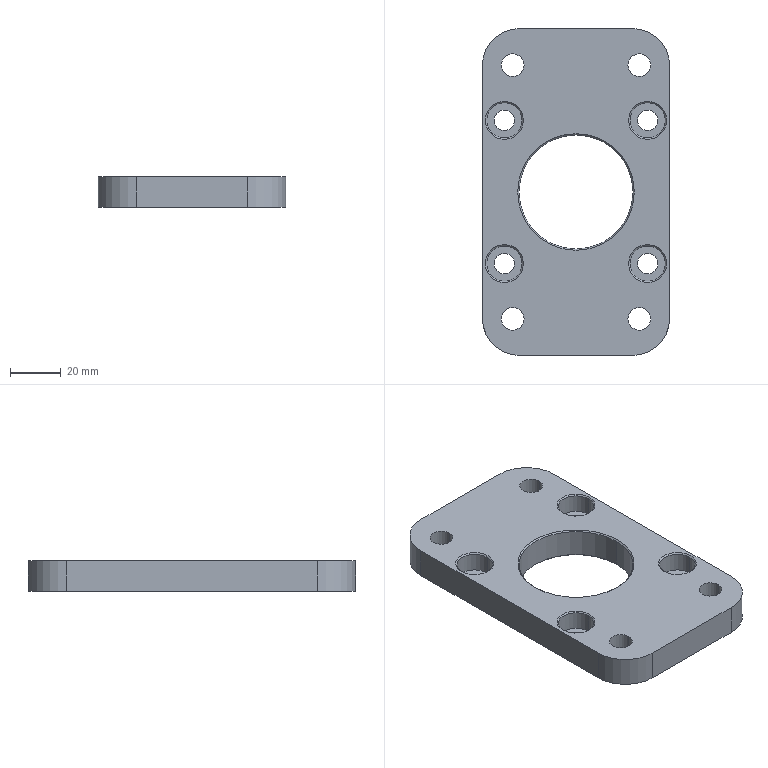Part | NX | 1 solid | 52 faces | box 74 x 129 x 12 mm | volume 84307 mm3 | cylinder 30 | cone 12 | plane 10 | commonest cylinder face diameters 8 x8 9 x8 14 x8 30 x4 45 x2
STEP:
#1=CARTESIAN_POINT('',(-35.25,28.25,11.5));
#2=VERTEX_POINT('',#1);
#3=CARTESIAN_POINT('',(-21.25,28.25,11.5));
#4=VERTEX_POINT('',#3);
#5=CARTESIAN_POINT('',(-28.25,28.25,11.5));
#6=DIRECTION('',(0.,0.,1.));
#7=DIRECTION('',(-1.,0.,0.));
#8=AXIS2_PLACEMENT_3D('',#5,#6,#7);
#9=CIRCLE('',#8,7.);
#10=EDGE_CURVE('',#2,#4,#9,.T.);
#11=ORIENTED_EDGE('',*,*,#10,.F.);
#12=CARTESIAN_POINT('',(-35.75,28.25,12.));
#13=VERTEX_POINT('',#12);
#14=CARTESIAN_POINT('',(-35.25,28.25,11.5));
#15=DIRECTION('',(-0.7071,0.,0.7071));
#16=VECTOR('',#15,1.);
#17=LINE('',#14,#16);
#18=EDGE_CURVE('',#2,#13,#17,.T.);
#19=ORIENTED_EDGE('',*,*,#18,.T.);
#20=CARTESIAN_POINT('',(-20.75,28.25,12.));
#21=VERTEX_POINT('',#20);
#22=CARTESIAN_POINT('',(-28.25,28.25,12.));
#23=DIRECTION('',(0.,0.,-1.));
#24=DIRECTION('',(-1.,0.,0.));
#25=AXIS2_PLACEMENT_3D('',#22,#23,#24);
#26=CIRCLE('',#25,7.5);
#27=EDGE_CURVE('',#21,#13,#26,.T.);
#28=ORIENTED_EDGE('',*,*,#27,.F.);
#29=CARTESIAN_POINT('',(-21.25,28.25,11.5));
#30=DIRECTION('',(0.7071,0.,0.7071));
#31=VECTOR('',#30,1.);
#32=LINE('',#29,#31);
#33=EDGE_CURVE('',#4,#21,#32,.T.);
#34=ORIENTED_EDGE('',*,*,#33,.F.);
#35=EDGE_LOOP('',(#11,#19,#28,#34));
#36=FACE_OUTER_BOUND('',#35,.T.);
#37=CARTESIAN_POINT('',(-28.25,28.25,11.5));
#38=DIRECTION('',(0.,0.,1.));
#39=DIRECTION('',(1.,0.,0.));
#40=AXIS2_PLACEMENT_3D('',#37,#38,#39);
#41=CONICAL_SURFACE('',#40,7.,45.);
#42=ADVANCED_FACE('',(#36),#41,.F.);
#43=CARTESIAN_POINT('',(21.25,28.25,11.5));
#44=VERTEX_POINT('',#43);
#45=CARTESIAN_POINT('',(35.25,28.25,11.5));
#46=VERTEX_POINT('',#45);
#47=CARTESIAN_POINT('',(28.25,28.25,11.5));
#48=DIRECTION('',(0.,0.,1.));
#49=DIRECTION('',(-1.,0.,0.));
#50=AXIS2_PLACEMENT_3D('',#47,#48,#49);
#51=CIRCLE('',#50,7.);
#52=EDGE_CURVE('',#44,#46,#51,.T.);
#53=ORIENTED_EDGE('',*,*,#52,.F.);
#54=CARTESIAN_POINT('',(20.75,28.25,12.));
#55=VERTEX_POINT('',#54);
#56=CARTESIAN_POINT('',(21.25,28.25,11.5));
#57=DIRECTION('',(-0.7071,0.,0.7071));
#58=VECTOR('',#57,1.);
#59=LINE('',#56,#58);
#60=EDGE_CURVE('',#44,#55,#59,.T.);
#61=ORIENTED_EDGE('',*,*,#60,.T.);
#62=CARTESIAN_POINT('',(35.75,28.25,12.));
#63=VERTEX_POINT('',#62);
#64=CARTESIAN_POINT('',(28.25,28.25,12.));
#65=DIRECTION('',(0.,0.,-1.));
#66=DIRECTION('',(-1.,0.,0.));
#67=AXIS2_PLACEMENT_3D('',#64,#65,#66);
#68=CIRCLE('',#67,7.5);
#69=EDGE_CURVE('',#63,#55,#68,.T.);
#70=ORIENTED_EDGE('',*,*,#69,.F.);
#71=CARTESIAN_POINT('',(35.25,28.25,11.5));
#72=DIRECTION('',(0.7071,0.,0.7071));
#73=VECTOR('',#72,1.);
#74=LINE('',#71,#73);
#75=EDGE_CURVE('',#46,#63,#74,.T.);
#76=ORIENTED_EDGE('',*,*,#75,.F.);
#77=EDGE_LOOP('',(#53,#61,#70,#76));
#78=FACE_OUTER_BOUND('',#77,.T.);
#79=CARTESIAN_POINT('',(28.25,28.25,11.5));
#80=DIRECTION('',(0.,0.,1.));
#81=DIRECTION('',(1.,0.,0.));
#82=AXIS2_PLACEMENT_3D('',#79,#80,#81);
#83=CONICAL_SURFACE('',#82,7.,45.);
#84=ADVANCED_FACE('',(#78),#83,.F.);
#85=CARTESIAN_POINT('',(21.25,-28.25,11.5));
#86=VERTEX_POINT('',#85);
#87=CARTESIAN_POINT('',(35.25,-28.25,11.5));
#88=VERTEX_POINT('',#87);
#89=CARTESIAN_POINT('',(28.25,-28.25,11.5));
#90=DIRECTION('',(0.,0.,1.));
#91=DIRECTION('',(-1.,0.,0.));
#92=AXIS2_PLACEMENT_3D('',#89,#90,#91);
#93=CIRCLE('',#92,7.);
#94=EDGE_CURVE('',#86,#88,#93,.T.);
#95=ORIENTED_EDGE('',*,*,#94,.F.);
#96=CARTESIAN_POINT('',(20.75,-28.25,12.));
#97=VERTEX_POINT('',#96);
#98=CARTESIAN_POINT('',(21.25,-28.25,11.5));
#99=DIRECTION('',(-0.7071,0.,0.7071));
#100=VECTOR('',#99,1.);
#101=LINE('',#98,#100);
#102=EDGE_CURVE('',#86,#97,#101,.T.);
#103=ORIENTED_EDGE('',*,*,#102,.T.);
#104=CARTESIAN_POINT('',(35.75,-28.25,12.));
#105=VERTEX_POINT('',#104);
#106=CARTESIAN_POINT('',(28.25,-28.25,12.));
#107=DIRECTION('',(0.,0.,-1.));
#108=DIRECTION('',(-1.,0.,0.));
#109=AXIS2_PLACEMENT_3D('',#106,#107,#108);
#110=CIRCLE('',#109,7.5);
#111=EDGE_CURVE('',#105,#97,#110,.T.);
#112=ORIENTED_EDGE('',*,*,#111,.F.);
#113=CARTESIAN_POINT('',(35.25,-28.25,11.5));
#114=DIRECTION('',(0.7071,0.,0.7071));
#115=VECTOR('',#114,1.);
#116=LINE('',#113,#115);
#117=EDGE_CURVE('',#88,#105,#116,.T.);
#118=ORIENTED_EDGE('',*,*,#117,.F.);
#119=EDGE_LOOP('',(#95,#103,#112,#118));
#120=FACE_OUTER_BOUND('',#119,.T.);
#121=CARTESIAN_POINT('',(28.25,-28.25,11.5));
#122=DIRECTION('',(0.,0.,1.));
#123=DIRECTION('',(1.,0.,0.));
#124=AXIS2_PLACEMENT_3D('',#121,#122,#123);
#125=CONICAL_SURFACE('',#124,7.,45.);
#126=ADVANCED_FACE('',(#120),#125,.F.);
#127=CARTESIAN_POINT('',(-35.25,-28.25,11.5));
#128=VERTEX_POINT('',#127);
#129=CARTESIAN_POINT('',(-21.25,-28.25,11.5));
#130=VERTEX_POINT('',#129);
#131=CARTESIAN_POINT('',(-28.25,-28.25,11.5));
#132=DIRECTION('',(0.,0.,1.));
#133=DIRECTION('',(-1.,0.,0.));
#134=AXIS2_PLACEMENT_3D('',#131,#132,#133);
#135=CIRCLE('',#134,7.);
#136=EDGE_CURVE('',#128,#130,#135,.T.);
#137=ORIENTED_EDGE('',*,*,#136,.F.);
#138=CARTESIAN_POINT('',(-35.75,-28.25,12.));
#139=VERTEX_POINT('',#138);
#140=CARTESIAN_POINT('',(-35.25,-28.25,11.5));
#141=DIRECTION('',(-0.7071,0.,0.7071));
#142=VECTOR('',#141,1.);
#143=LINE('',#140,#142);
#144=EDGE_CURVE('',#128,#139,#143,.T.);
#145=ORIENTED_EDGE('',*,*,#144,.T.);
#146=CARTESIAN_POINT('',(-20.75,-28.25,12.));
#147=VERTEX_POINT('',#146);
#148=CARTESIAN_POINT('',(-28.25,-28.25,12.));
#149=DIRECTION('',(0.,0.,-1.));
#150=DIRECTION('',(-1.,0.,0.));
#151=AXIS2_PLACEMENT_3D('',#148,#149,#150);
#152=CIRCLE('',#151,7.5);
#153=EDGE_CURVE('',#147,#139,#152,.T.);
#154=ORIENTED_EDGE('',*,*,#153,.F.);
#155=CARTESIAN_POINT('',(-21.25,-28.25,11.5));
#156=DIRECTION('',(0.7071,0.,0.7071));
#157=VECTOR('',#156,1.);
#158=LINE('',#155,#157);
#159=EDGE_CURVE('',#130,#147,#158,.T.);
#160=ORIENTED_EDGE('',*,*,#159,.F.);
#161=EDGE_LOOP('',(#137,#145,#154,#160));
#162=FACE_OUTER_BOUND('',#161,.T.);
#163=CARTESIAN_POINT('',(-28.25,-28.25,11.5));
#164=DIRECTION('',(0.,0.,1.));
#165=DIRECTION('',(1.,0.,0.));
#166=AXIS2_PLACEMENT_3D('',#163,#164,#165);
#167=CONICAL_SURFACE('',#166,7.,45.);
#168=ADVANCED_FACE('',(#162),#167,.F.);
#169=CARTESIAN_POINT('',(-22.5,0.,11.5));
#170=VERTEX_POINT('',#169);
#171=CARTESIAN_POINT('',(22.5,0.,11.5));
#172=VERTEX_POINT('',#171);
#173=CARTESIAN_POINT('',(0.,0.,11.5));
#174=DIRECTION('',(0.,0.,1.));
#175=DIRECTION('',(-1.,0.,0.));
#176=AXIS2_PLACEMENT_3D('',#173,#174,#175);
#177=CIRCLE('',#176,22.5);
#178=EDGE_CURVE('',#170,#172,#177,.T.);
#179=ORIENTED_EDGE('',*,*,#178,.F.);
#180=CARTESIAN_POINT('',(-23.,0.,12.));
#181=VERTEX_POINT('',#180);
#182=CARTESIAN_POINT('',(-22.5,0.,11.5));
#183=DIRECTION('',(-0.7071,0.,0.7071));
#184=VECTOR('',#183,1.);
#185=LINE('',#182,#184);
#186=EDGE_CURVE('',#170,#181,#185,.T.);
#187=ORIENTED_EDGE('',*,*,#186,.T.);
#188=CARTESIAN_POINT('',(23.,0.,12.));
#189=VERTEX_POINT('',#188);
#190=CARTESIAN_POINT('',(0.,0.,12.));
#191=DIRECTION('',(0.,0.,-1.));
#192=DIRECTION('',(-1.,0.,0.));
#193=AXIS2_PLACEMENT_3D('',#190,#191,#192);
#194=CIRCLE('',#193,23.);
#195=EDGE_CURVE('',#189,#181,#194,.T.);
#196=ORIENTED_EDGE('',*,*,#195,.F.);
#197=CARTESIAN_POINT('',(22.5,0.,11.5));
#198=DIRECTION('',(0.7071,0.,0.7071));
#199=VECTOR('',#198,1.);
#200=LINE('',#197,#199);
#201=EDGE_CURVE('',#172,#189,#200,.T.);
#202=ORIENTED_EDGE('',*,*,#201,.F.);
#203=EDGE_LOOP('',(#179,#187,#196,#202));
#204=FACE_OUTER_BOUND('',#203,.T.);
#205=CARTESIAN_POINT('',(0.,0.,11.5));
#206=DIRECTION('',(0.,0.,1.));
#207=DIRECTION('',(1.,0.,0.));
#208=AXIS2_PLACEMENT_3D('',#205,#206,#207);
#209=CONICAL_SURFACE('',#208,22.5,45.);
#210=ADVANCED_FACE('',(#204),#209,.F.);
#211=CARTESIAN_POINT('',(22.5,0.,0.5));
#212=VERTEX_POINT('',#211);
#213=CARTESIAN_POINT('',(-22.5,0.,0.5));
#214=VERTEX_POINT('',#213);
#215=CARTESIAN_POINT('',(0.,0.,0.5));
#216=DIRECTION('',(0.,0.,-1.));
#217=DIRECTION('',(-1.,0.,0.));
#218=AXIS2_PLACEMENT_3D('',#215,#216,#217);
#219=CIRCLE('',#218,22.5);
#220=EDGE_CURVE('',#212,#214,#219,.T.);
#221=ORIENTED_EDGE('',*,*,#220,.F.);
#222=CARTESIAN_POINT('',(23.,0.,0.));
#223=VERTEX_POINT('',#222);
#224=CARTESIAN_POINT('',(23.,0.,0.));
#225=DIRECTION('',(-0.7071,0.,0.7071));
#226=VECTOR('',#225,1.);
#227=LINE('',#224,#226);
#228=EDGE_CURVE('',#223,#212,#227,.T.);
#229=ORIENTED_EDGE('',*,*,#228,.F.);
#230=CARTESIAN_POINT('',(-23.,0.,0.));
#231=VERTEX_POINT('',#230);
#232=CARTESIAN_POINT('',(0.,0.,0.));
#233=DIRECTION('',(0.,0.,1.));
#234=DIRECTION('',(-1.,0.,0.));
#235=AXIS2_PLACEMENT_3D('',#232,#233,#234);
#236=CIRCLE('',#235,23.);
#237=EDGE_CURVE('',#231,#223,#236,.T.);
#238=ORIENTED_EDGE('',*,*,#237,.F.);
#239=CARTESIAN_POINT('',(-23.,0.,0.));
#240=DIRECTION('',(0.7071,0.,0.7071));
#241=VECTOR('',#240,1.);
#242=LINE('',#239,#241);
#243=EDGE_CURVE('',#231,#214,#242,.T.);
#244=ORIENTED_EDGE('',*,*,#243,.T.);
#245=EDGE_LOOP('',(#221,#229,#238,#244));
#246=FACE_OUTER_BOUND('',#245,.T.);
#247=CARTESIAN_POINT('',(0.,0.,0.));
#248=DIRECTION('',(0.,0.,-1.));
#249=DIRECTION('',(-1.,0.,0.));
#250=AXIS2_PLACEMENT_3D('',#247,#248,#249);
#251=CONICAL_SURFACE('',#250,23.,45.);
#252=ADVANCED_FACE('',(#246),#251,.F.);
#253=CARTESIAN_POINT('',(21.25,-28.25,4.));
#254=VERTEX_POINT('',#253);
#255=CARTESIAN_POINT('',(35.25,-28.25,4.));
#256=VERTEX_POINT('',#255);
#257=CARTESIAN_POINT('',(28.25,-28.25,4.));
#258=DIRECTION('',(0.,0.,1.));
#259=DIRECTION('',(1.,0.,0.));
#260=AXIS2_PLACEMENT_3D('',#257,#258,#259);
#261=CIRCLE('',#260,7.);
#262=EDGE_CURVE('',#254,#256,#261,.T.);
#263=ORIENTED_EDGE('',*,*,#262,.F.);
#264=CARTESIAN_POINT('',(21.25,-28.25,4.));
#265=DIRECTION('',(0.,0.,1.));
#266=VECTOR('',#265,1.);
#267=LINE('',#264,#266);
#268=EDGE_CURVE('',#254,#86,#267,.T.);
#269=ORIENTED_EDGE('',*,*,#268,.T.);
#270=ORIENTED_EDGE('',*,*,#94,.T.);
#271=CARTESIAN_POINT('',(35.25,-28.25,4.));
#272=DIRECTION('',(0.,0.,1.));
#273=VECTOR('',#272,1.);
#274=LINE('',#271,#273);
#275=EDGE_CURVE('',#256,#88,#274,.T.);
#276=ORIENTED_EDGE('',*,*,#275,.F.);
#277=EDGE_LOOP('',(#263,#269,#270,#276));
#278=FACE_OUTER_BOUND('',#277,.T.);
#279=CARTESIAN_POINT('',(28.25,-28.25,4.));
#280=DIRECTION('',(0.,0.,1.));
#281=DIRECTION('',(1.,0.,0.));
#282=AXIS2_PLACEMENT_3D('',#279,#280,#281);
#283=CYLINDRICAL_SURFACE('',#282,7.);
#284=ADVANCED_FACE('',(#278),#283,.F.);
#285=CARTESIAN_POINT('',(-35.25,-28.25,4.));
#286=VERTEX_POINT('',#285);
#287=CARTESIAN_POINT('',(-21.25,-28.25,4.));
#288=VERTEX_POINT('',#287);
#289=CARTESIAN_POINT('',(-28.25,-28.25,4.));
#290=DIRECTION('',(0.,0.,1.));
#291=DIRECTION('',(1.,0.,0.));
#292=AXIS2_PLACEMENT_3D('',#289,#290,#291);
#293=CIRCLE('',#292,7.);
#294=EDGE_CURVE('',#286,#288,#293,.T.);
#295=ORIENTED_EDGE('',*,*,#294,.F.);
#296=CARTESIAN_POINT('',(-35.25,-28.25,4.));
#297=DIRECTION('',(0.,0.,1.));
#298=VECTOR('',#297,1.);
#299=LINE('',#296,#298);
#300=EDGE_CURVE('',#286,#128,#299,.T.);
#301=ORIENTED_EDGE('',*,*,#300,.T.);
#302=ORIENTED_EDGE('',*,*,#136,.T.);
#303=CARTESIAN_POINT('',(-21.25,-28.25,4.));
#304=DIRECTION('',(0.,0.,1.));
#305=VECTOR('',#304,1.);
#306=LINE('',#303,#305);
#307=EDGE_CURVE('',#288,#130,#306,.T.);
#308=ORIENTED_EDGE('',*,*,#307,.F.);
#309=EDGE_LOOP('',(#295,#301,#302,#308));
#310=FACE_OUTER_BOUND('',#309,.T.);
#311=CARTESIAN_POINT('',(-28.25,-28.25,4.));
#312=DIRECTION('',(0.,0.,1.));
#313=DIRECTION('',(1.,0.,0.));
#314=AXIS2_PLACEMENT_3D('',#311,#312,#313);
#315=CYLINDRICAL_SURFACE('',#314,7.);
#316=ADVANCED_FACE('',(#310),#315,.F.);
#317=CARTESIAN_POINT('',(21.25,28.25,4.));
#318=VERTEX_POINT('',#317);
#319=CARTESIAN_POINT('',(35.25,28.25,4.));
#320=VERTEX_POINT('',#319);
#321=CARTESIAN_POINT('',(28.25,28.25,4.));
#322=DIRECTION('',(0.,0.,1.));
#323=DIRECTION('',(1.,0.,0.));
#324=AXIS2_PLACEMENT_3D('',#321,#322,#323);
#325=CIRCLE('',#324,7.);
#326=EDGE_CURVE('',#318,#320,#325,.T.);
#327=ORIENTED_EDGE('',*,*,#326,.F.);
#328=CARTESIAN_POINT('',(21.25,28.25,4.));
#329=DIRECTION('',(0.,0.,1.));
#330=VECTOR('',#329,1.);
#331=LINE('',#328,#330);
#332=EDGE_CURVE('',#318,#44,#331,.T.);
#333=ORIENTED_EDGE('',*,*,#332,.T.);
#334=ORIENTED_EDGE('',*,*,#52,.T.);
#335=CARTESIAN_POINT('',(35.25,28.25,4.));
#336=DIRECTION('',(0.,0.,1.));
#337=VECTOR('',#336,1.);
#338=LINE('',#335,#337);
#339=EDGE_CURVE('',#320,#46,#338,.T.);
#340=ORIENTED_EDGE('',*,*,#339,.F.);
#341=EDGE_LOOP('',(#327,#333,#334,#340));
#342=FACE_OUTER_BOUND('',#341,.T.);
#343=CARTESIAN_POINT('',(28.25,28.25,4.));
#344=DIRECTION('',(0.,0.,1.));
#345=DIRECTION('',(1.,0.,0.));
#346=AXIS2_PLACEMENT_3D('',#343,#344,#345);
#347=CYLINDRICAL_SURFACE('',#346,7.);
#348=ADVANCED_FACE('',(#342),#347,.F.);
#349=CARTESIAN_POINT('',(-35.25,28.25,4.));
#350=VERTEX_POINT('',#349);
#351=CARTESIAN_POINT('',(-21.25,28.25,4.));
#352=VERTEX_POINT('',#351);
#353=CARTESIAN_POINT('',(-28.25,28.25,4.));
#354=DIRECTION('',(0.,0.,1.));
#355=DIRECTION('',(1.,0.,0.));
#356=AXIS2_PLACEMENT_3D('',#353,#354,#355);
#357=CIRCLE('',#356,7.);
#358=EDGE_CURVE('',#350,#352,#357,.T.);
#359=ORIENTED_EDGE('',*,*,#358,.F.);
#360=CARTESIAN_POINT('',(-35.25,28.25,4.));
#361=DIRECTION('',(0.,0.,1.));
#362=VECTOR('',#361,1.);
#363=LINE('',#360,#362);
#364=EDGE_CURVE('',#350,#2,#363,.T.);
#365=ORIENTED_EDGE('',*,*,#364,.T.);
#366=ORIENTED_EDGE('',*,*,#10,.T.);
#367=CARTESIAN_POINT('',(-21.25,28.25,4.));
#368=DIRECTION('',(0.,0.,1.));
#369=VECTOR('',#368,1.);
#370=LINE('',#367,#369);
#371=EDGE_CURVE('',#352,#4,#370,.T.);
#372=ORIENTED_EDGE('',*,*,#371,.F.);
#373=EDGE_LOOP('',(#359,#365,#366,#372));
#374=FACE_OUTER_BOUND('',#373,.T.);
#375=CARTESIAN_POINT('',(-28.25,28.25,4.));
#376=DIRECTION('',(0.,0.,1.));
#377=DIRECTION('',(1.,0.,0.));
#378=AXIS2_PLACEMENT_3D('',#375,#376,#377);
#379=CYLINDRICAL_SURFACE('',#378,7.);
#380=ADVANCED_FACE('',(#374),#379,.F.);
#381=CARTESIAN_POINT('',(-29.5,50.,0.));
#382=VERTEX_POINT('',#381);
#383=CARTESIAN_POINT('',(-20.5,50.,0.));
#384=VERTEX_POINT('',#383);
#385=CARTESIAN_POINT('',(-25.,50.,0.));
#386=DIRECTION('',(0.,0.,1.));
#387=DIRECTION('',(-1.,0.,0.));
#388=AXIS2_PLACEMENT_3D('',#385,#386,#387);
#389=CIRCLE('',#388,4.5);
#390=EDGE_CURVE('',#382,#384,#389,.T.);
#391=ORIENTED_EDGE('',*,*,#390,.F.);
#392=CARTESIAN_POINT('',(-29.5,50.,12.));
#393=VERTEX_POINT('',#392);
#394=CARTESIAN_POINT('',(-29.5,50.,12.));
#395=DIRECTION('',(0.,0.,1.));
#396=VECTOR('',#395,1.);
#397=LINE('',#394,#396);
#398=EDGE_CURVE('',#382,#393,#397,.T.);
#399=ORIENTED_EDGE('',*,*,#398,.T.);
#400=CARTESIAN_POINT('',(-20.5,50.,12.));
#401=VERTEX_POINT('',#400);
#402=CARTESIAN_POINT('',(-25.,50.,12.));
#403=DIRECTION('',(0.,0.,1.));
#404=DIRECTION('',(1.,0.,0.));
#405=AXIS2_PLACEMENT_3D('',#402,#403,#404);
#406=CIRCLE('',#405,4.5);
#407=EDGE_CURVE('',#393,#401,#406,.T.);
#408=ORIENTED_EDGE('',*,*,#407,.T.);
#409=CARTESIAN_POINT('',(-20.5,50.,12.));
#410=DIRECTION('',(0.,0.,1.));
#411=VECTOR('',#410,1.);
#412=LINE('',#409,#411);
#413=EDGE_CURVE('',#384,#401,#412,.T.);
#414=ORIENTED_EDGE('',*,*,#413,.F.);
#415=EDGE_LOOP('',(#391,#399,#408,#414));
#416=FACE_OUTER_BOUND('',#415,.T.);
#417=CARTESIAN_POINT('',(-25.,50.,12.));
#418=DIRECTION('',(0.,0.,1.));
#419=DIRECTION('',(1.,0.,0.));
#420=AXIS2_PLACEMENT_3D('',#417,#418,#419);
#421=CYLINDRICAL_SURFACE('',#420,4.5);
#422=ADVANCED_FACE('',(#416),#421,.F.);
#423=CARTESIAN_POINT('',(20.5,50.,0.));
#424=VERTEX_POINT('',#423);
#425=CARTESIAN_POINT('',(29.5,50.,0.));
#426=VERTEX_POINT('',#425);
#427=CARTESIAN_POINT('',(25.,50.,0.));
#428=DIRECTION('',(0.,0.,1.));
#429=DIRECTION('',(-1.,0.,0.));
#430=AXIS2_PLACEMENT_3D('',#427,#428,#429);
#431=CIRCLE('',#430,4.5);
#432=EDGE_CURVE('',#424,#426,#431,.T.);
#433=ORIENTED_EDGE('',*,*,#432,.F.);
#434=CARTESIAN_POINT('',(20.5,50.,12.));
#435=VERTEX_POINT('',#434);
#436=CARTESIAN_POINT('',(20.5,50.,12.));
#437=DIRECTION('',(0.,0.,1.));
#438=VECTOR('',#437,1.);
#439=LINE('',#436,#438);
#440=EDGE_CURVE('',#424,#435,#439,.T.);
#441=ORIENTED_EDGE('',*,*,#440,.T.);
#442=CARTESIAN_POINT('',(29.5,50.,12.));
#443=VERTEX_POINT('',#442);
#444=CARTESIAN_POINT('',(25.,50.,12.));
#445=DIRECTION('',(0.,0.,1.));
#446=DIRECTION('',(1.,0.,0.));
#447=AXIS2_PLACEMENT_3D('',#444,#445,#446);
#448=CIRCLE('',#447,4.5);
#449=EDGE_CURVE('',#435,#443,#448,.T.);
#450=ORIENTED_EDGE('',*,*,#449,.T.);
#451=CARTESIAN_POINT('',(29.5,50.,12.));
#452=DIRECTION('',(0.,0.,1.));
#453=VECTOR('',#452,1.);
#454=LINE('',#451,#453);
#455=EDGE_CURVE('',#426,#443,#454,.T.);
#456=ORIENTED_EDGE('',*,*,#455,.F.);
#457=EDGE_LOOP('',(#433,#441,#450,#456));
#458=FACE_OUTER_BOUND('',#457,.T.);
#459=CARTESIAN_POINT('',(25.,50.,12.));
#460=DIRECTION('',(0.,0.,1.));
#461=DIRECTION('',(1.,0.,0.));
#462=AXIS2_PLACEMENT_3D('',#459,#460,#461);
#463=CYLINDRICAL_SURFACE('',#462,4.5);
#464=ADVANCED_FACE('',(#458),#463,.F.);
#465=CARTESIAN_POINT('',(-29.5,-50.,0.));
#466=VERTEX_POINT('',#465);
#467=CARTESIAN_POINT('',(-20.5,-50.,0.));
#468=VERTEX_POINT('',#467);
#469=CARTESIAN_POINT('',(-25.,-50.,0.));
#470=DIRECTION('',(0.,0.,1.));
#471=DIRECTION('',(-1.,0.,0.));
#472=AXIS2_PLACEMENT_3D('',#469,#470,#471);
#473=CIRCLE('',#472,4.5);
#474=EDGE_CURVE('',#466,#468,#473,.T.);
#475=ORIENTED_EDGE('',*,*,#474,.F.);
#476=CARTESIAN_POINT('',(-29.5,-50.,12.));
#477=VERTEX_POINT('',#476);
#478=CARTESIAN_POINT('',(-29.5,-50.,12.));
#479=DIRECTION('',(0.,0.,1.));
#480=VECTOR('',#479,1.);
#481=LINE('',#478,#480);
#482=EDGE_CURVE('',#466,#477,#481,.T.);
#483=ORIENTED_EDGE('',*,*,#482,.T.);
#484=CARTESIAN_POINT('',(-20.5,-50.,12.));
#485=VERTEX_POINT('',#484);
#486=CARTESIAN_POINT('',(-25.,-50.,12.));
#487=DIRECTION('',(0.,0.,1.));
#488=DIRECTION('',(1.,0.,0.));
#489=AXIS2_PLACEMENT_3D('',#486,#487,#488);
#490=CIRCLE('',#489,4.5);
#491=EDGE_CURVE('',#477,#485,#490,.T.);
#492=ORIENTED_EDGE('',*,*,#491,.T.);
#493=CARTESIAN_POINT('',(-20.5,-50.,12.));
#494=DIRECTION('',(0.,0.,1.));
#495=VECTOR('',#494,1.);
#496=LINE('',#493,#495);
#497=EDGE_CURVE('',#468,#485,#496,.T.);
#498=ORIENTED_EDGE('',*,*,#497,.F.);
#499=EDGE_LOOP('',(#475,#483,#492,#498));
#500=FACE_OUTER_BOUND('',#499,.T.);
#501=CARTESIAN_POINT('',(-25.,-50.,12.));
#502=DIRECTION('',(0.,0.,1.));
#503=DIRECTION('',(1.,0.,0.));
#504=AXIS2_PLACEMENT_3D('',#501,#502,#503);
#505=CYLINDRICAL_SURFACE('',#504,4.5);
#506=ADVANCED_FACE('',(#500),#505,.F.);
#507=CARTESIAN_POINT('',(20.5,-50.,0.));
#508=VERTEX_POINT('',#507);
#509=CARTESIAN_POINT('',(29.5,-50.,0.));
#510=VERTEX_POINT('',#509);
#511=CARTESIAN_POINT('',(25.,-50.,0.));
#512=DIRECTION('',(0.,0.,1.));
#513=DIRECTION('',(-1.,0.,0.));
#514=AXIS2_PLACEMENT_3D('',#511,#512,#513);
#515=CIRCLE('',#514,4.5);
#516=EDGE_CURVE('',#508,#510,#515,.T.);
#517=ORIENTED_EDGE('',*,*,#516,.F.);
#518=CARTESIAN_POINT('',(20.5,-50.,12.));
#519=VERTEX_POINT('',#518);
#520=CARTESIAN_POINT('',(20.5,-50.,12.));
#521=DIRECTION('',(0.,0.,1.));
#522=VECTOR('',#521,1.);
#523=LINE('',#520,#522);
#524=EDGE_CURVE('',#508,#519,#523,.T.);
#525=ORIENTED_EDGE('',*,*,#524,.T.);
#526=CARTESIAN_POINT('',(29.5,-50.,12.));
#527=VERTEX_POINT('',#526);
#528=CARTESIAN_POINT('',(25.,-50.,12.));
#529=DIRECTION('',(0.,0.,1.));
#530=DIRECTION('',(1.,0.,0.));
#531=AXIS2_PLACEMENT_3D('',#528,#529,#530);
#532=CIRCLE('',#531,4.5);
#533=EDGE_CURVE('',#519,#527,#532,.T.);
#534=ORIENTED_EDGE('',*,*,#533,.T.);
#535=CARTESIAN_POINT('',(29.5,-50.,12.));
#536=DIRECTION('',(0.,0.,1.));
#537=VECTOR('',#536,1.);
#538=LINE('',#535,#537);
#539=EDGE_CURVE('',#510,#527,#538,.T.);
#540=ORIENTED_EDGE('',*,*,#539,.F.);
#541=EDGE_LOOP('',(#517,#525,#534,#540));
#542=FACE_OUTER_BOUND('',#541,.T.);
#543=CARTESIAN_POINT('',(25.,-50.,12.));
#544=DIRECTION('',(0.,0.,1.));
#545=DIRECTION('',(1.,0.,0.));
#546=AXIS2_PLACEMENT_3D('',#543,#544,#545);
#547=CYLINDRICAL_SURFACE('',#546,4.5);
#548=ADVANCED_FACE('',(#542),#547,.F.);
#549=ORIENTED_EDGE('',*,*,#178,.T.);
#550=CARTESIAN_POINT('',(22.5,0.,12.));
#551=DIRECTION('',(0.,0.,1.));
#552=VECTOR('',#551,1.);
#553=LINE('',#550,#552);
#554=EDGE_CURVE('',#212,#172,#553,.T.);
#555=ORIENTED_EDGE('',*,*,#554,.F.);
#556=ORIENTED_EDGE('',*,*,#220,.T.);
#557=CARTESIAN_POINT('',(-22.5,0.,12.));
#558=DIRECTION('',(0.,0.,1.));
#559=VECTOR('',#558,1.);
#560=LINE('',#557,#559);
#561=EDGE_CURVE('',#214,#170,#560,.T.);
#562=ORIENTED_EDGE('',*,*,#561,.T.);
#563=EDGE_LOOP('',(#549,#555,#556,#562));
#564=FACE_OUTER_BOUND('',#563,.T.);
#565=CARTESIAN_POINT('',(0.,0.,12.));
#566=DIRECTION('',(0.,0.,-1.));
#567=DIRECTION('',(-1.,0.,0.));
#568=AXIS2_PLACEMENT_3D('',#565,#566,#567);
#569=CYLINDRICAL_SURFACE('',#568,22.5);
#570=ADVANCED_FACE('',(#564),#569,.F.);
#571=CARTESIAN_POINT('',(-32.25,28.25,0.));
#572=VERTEX_POINT('',#571);
#573=CARTESIAN_POINT('',(-24.25,28.25,0.));
#574=VERTEX_POINT('',#573);
#575=CARTESIAN_POINT('',(-28.25,28.25,0.));
#576=DIRECTION('',(0.,0.,1.));
#577=DIRECTION('',(-1.,0.,0.));
#578=AXIS2_PLACEMENT_3D('',#575,#576,#577);
#579=CIRCLE('',#578,4.);
#580=EDGE_CURVE('',#572,#574,#579,.T.);
#581=ORIENTED_EDGE('',*,*,#580,.F.);
#582=CARTESIAN_POINT('',(-32.25,28.25,4.));
#583=VERTEX_POINT('',#582);
#584=CARTESIAN_POINT('',(-32.25,28.25,-11.314));
#585=DIRECTION('',(0.,0.,1.));
#586=VECTOR('',#585,1.);
#587=LINE('',#584,#586);
#588=EDGE_CURVE('',#572,#583,#587,.T.);
#589=ORIENTED_EDGE('',*,*,#588,.T.);
#590=CARTESIAN_POINT('',(-24.25,28.25,4.));
#591=VERTEX_POINT('',#590);
#592=CARTESIAN_POINT('',(-28.25,28.25,4.));
#593=DIRECTION('',(0.,0.,-1.));
#594=DIRECTION('',(1.,0.,0.));
#595=AXIS2_PLACEMENT_3D('',#592,#593,#594);
#596=CIRCLE('',#595,4.);
#597=EDGE_CURVE('',#591,#583,#596,.T.);
#598=ORIENTED_EDGE('',*,*,#597,.F.);
#599=CARTESIAN_POINT('',(-24.25,28.25,-11.314));
#600=DIRECTION('',(0.,0.,1.));
#601=VECTOR('',#600,1.);
#602=LINE('',#599,#601);
#603=EDGE_CURVE('',#574,#591,#602,.T.);
#604=ORIENTED_EDGE('',*,*,#603,.F.);
#605=EDGE_LOOP('',(#581,#589,#598,#604));
#606=FACE_OUTER_BOUND('',#605,.T.);
#607=CARTESIAN_POINT('',(-28.25,28.25,-11.314));
#608=DIRECTION('',(0.,0.,1.));
#609=DIRECTION('',(1.,0.,0.));
#610=AXIS2_PLACEMENT_3D('',#607,#608,#609);
#611=CYLINDRICAL_SURFACE('',#610,4.);
#612=ADVANCED_FACE('',(#606),#611,.F.);
#613=CARTESIAN_POINT('',(24.25,28.25,0.));
#614=VERTEX_POINT('',#613);
#615=CARTESIAN_POINT('',(32.25,28.25,0.));
#616=VERTEX_POINT('',#615);
#617=CARTESIAN_POINT('',(28.25,28.25,0.));
#618=DIRECTION('',(0.,0.,1.));
#619=DIRECTION('',(-1.,0.,0.));
#620=AXIS2_PLACEMENT_3D('',#617,#618,#619);
#621=CIRCLE('',#620,4.);
#622=EDGE_CURVE('',#614,#616,#621,.T.);
#623=ORIENTED_EDGE('',*,*,#622,.F.);
#624=CARTESIAN_POINT('',(24.25,28.25,4.));
#625=VERTEX_POINT('',#624);
#626=CARTESIAN_POINT('',(24.25,28.25,-11.314));
#627=DIRECTION('',(0.,0.,1.));
#628=VECTOR('',#627,1.);
#629=LINE('',#626,#628);
#630=EDGE_CURVE('',#614,#625,#629,.T.);
#631=ORIENTED_EDGE('',*,*,#630,.T.);
#632=CARTESIAN_POINT('',(32.25,28.25,4.));
#633=VERTEX_POINT('',#632);
#634=CARTESIAN_POINT('',(28.25,28.25,4.));
#635=DIRECTION('',(0.,0.,-1.));
#636=DIRECTION('',(1.,0.,0.));
#637=AXIS2_PLACEMENT_3D('',#634,#635,#636);
#638=CIRCLE('',#637,4.);
#639=EDGE_CURVE('',#633,#625,#638,.T.);
#640=ORIENTED_EDGE('',*,*,#639,.F.);
#641=CARTESIAN_POINT('',(32.25,28.25,-11.314));
#642=DIRECTION('',(0.,0.,1.));
#643=VECTOR('',#642,1.);
#644=LINE('',#641,#643);
#645=EDGE_CURVE('',#616,#633,#644,.T.);
#646=ORIENTED_EDGE('',*,*,#645,.F.);
#647=EDGE_LOOP('',(#623,#631,#640,#646));
#648=FACE_OUTER_BOUND('',#647,.T.);
#649=CARTESIAN_POINT('',(28.25,28.25,-11.314));
#650=DIRECTION('',(0.,0.,1.));
#651=DIRECTION('',(1.,0.,0.));
#652=AXIS2_PLACEMENT_3D('',#649,#650,#651);
#653=CYLINDRICAL_SURFACE('',#652,4.);
#654=ADVANCED_FACE('',(#648),#653,.F.);
#655=CARTESIAN_POINT('',(-32.25,-28.25,0.));
#656=VERTEX_POINT('',#655);
#657=CARTESIAN_POINT('',(-24.25,-28.25,0.));
#658=VERTEX_POINT('',#657);
#659=CARTESIAN_POINT('',(-28.25,-28.25,0.));
#660=DIRECTION('',(0.,0.,1.));
#661=DIRECTION('',(-1.,0.,0.));
#662=AXIS2_PLACEMENT_3D('',#659,#660,#661);
#663=CIRCLE('',#662,4.);
#664=EDGE_CURVE('',#656,#658,#663,.T.);
#665=ORIENTED_EDGE('',*,*,#664,.F.);
#666=CARTESIAN_POINT('',(-32.25,-28.25,4.));
#667=VERTEX_POINT('',#666);
#668=CARTESIAN_POINT('',(-32.25,-28.25,-11.314));
#669=DIRECTION('',(0.,0.,1.));
#670=VECTOR('',#669,1.);
#671=LINE('',#668,#670);
#672=EDGE_CURVE('',#656,#667,#671,.T.);
#673=ORIENTED_EDGE('',*,*,#672,.T.);
#674=CARTESIAN_POINT('',(-24.25,-28.25,4.));
#675=VERTEX_POINT('',#674);
#676=CARTESIAN_POINT('',(-28.25,-28.25,4.));
#677=DIRECTION('',(0.,0.,-1.));
#678=DIRECTION('',(1.,0.,0.));
#679=AXIS2_PLACEMENT_3D('',#676,#677,#678);
#680=CIRCLE('',#679,4.);
#681=EDGE_CURVE('',#675,#667,#680,.T.);
#682=ORIENTED_EDGE('',*,*,#681,.F.);
#683=CARTESIAN_POINT('',(-24.25,-28.25,-11.314));
#684=DIRECTION('',(0.,0.,1.));
#685=VECTOR('',#684,1.);
#686=LINE('',#683,#685);
#687=EDGE_CURVE('',#658,#675,#686,.T.);
#688=ORIENTED_EDGE('',*,*,#687,.F.);
#689=EDGE_LOOP('',(#665,#673,#682,#688));
#690=FACE_OUTER_BOUND('',#689,.T.);
#691=CARTESIAN_POINT('',(-28.25,-28.25,-11.314));
#692=DIRECTION('',(0.,0.,1.));
#693=DIRECTION('',(1.,0.,0.));
#694=AXIS2_PLACEMENT_3D('',#691,#692,#693);
#695=CYLINDRICAL_SURFACE('',#694,4.);
#696=ADVANCED_FACE('',(#690),#695,.F.);
#697=CARTESIAN_POINT('',(24.25,-28.25,0.));
#698=VERTEX_POINT('',#697);
#699=CARTESIAN_POINT('',(32.25,-28.25,0.));
#700=VERTEX_POINT('',#699);
#701=CARTESIAN_POINT('',(28.25,-28.25,0.));
#702=DIRECTION('',(0.,0.,1.));
#703=DIRECTION('',(-1.,0.,0.));
#704=AXIS2_PLACEMENT_3D('',#701,#702,#703);
#705=CIRCLE('',#704,4.);
#706=EDGE_CURVE('',#698,#700,#705,.T.);
#707=ORIENTED_EDGE('',*,*,#706,.F.);
#708=CARTESIAN_POINT('',(24.25,-28.25,4.));
#709=VERTEX_POINT('',#708);
#710=CARTESIAN_POINT('',(24.25,-28.25,-11.314));
#711=DIRECTION('',(0.,0.,1.));
#712=VECTOR('',#711,1.);
#713=LINE('',#710,#712);
#714=EDGE_CURVE('',#698,#709,#713,.T.);
#715=ORIENTED_EDGE('',*,*,#714,.T.);
#716=CARTESIAN_POINT('',(32.25,-28.25,4.));
#717=VERTEX_POINT('',#716);
#718=CARTESIAN_POINT('',(28.25,-28.25,4.));
#719=DIRECTION('',(0.,0.,-1.));
#720=DIRECTION('',(1.,0.,0.));
#721=AXIS2_PLACEMENT_3D('',#718,#719,#720);
#722=CIRCLE('',#721,4.);
#723=EDGE_CURVE('',#717,#709,#722,.T.);
#724=ORIENTED_EDGE('',*,*,#723,.F.);
#725=CARTESIAN_POINT('',(32.25,-28.25,-11.314));
#726=DIRECTION('',(0.,0.,1.));
#727=VECTOR('',#726,1.);
#728=LINE('',#725,#727);
#729=EDGE_CURVE('',#700,#717,#728,.T.);
#730=ORIENTED_EDGE('',*,*,#729,.F.);
#731=EDGE_LOOP('',(#707,#715,#724,#730));
#732=FACE_OUTER_BOUND('',#731,.T.);
#733=CARTESIAN_POINT('',(28.25,-28.25,-11.314));
#734=DIRECTION('',(0.,0.,1.));
#735=DIRECTION('',(1.,0.,0.));
#736=AXIS2_PLACEMENT_3D('',#733,#734,#735);
#737=CYLINDRICAL_SURFACE('',#736,4.);
#738=ADVANCED_FACE('',(#732),#737,.F.);
#739=ORIENTED_EDGE('',*,*,#714,.F.);
#740=CARTESIAN_POINT('',(28.25,-28.25,0.));
#741=DIRECTION('',(0.,0.,1.));
#742=DIRECTION('',(-1.,0.,0.));
#743=AXIS2_PLACEMENT_3D('',#740,#741,#742);
#744=CIRCLE('',#743,4.);
#745=EDGE_CURVE('',#700,#698,#744,.T.);
#746=ORIENTED_EDGE('',*,*,#745,.F.);
#747=ORIENTED_EDGE('',*,*,#729,.T.);
#748=CARTESIAN_POINT('',(28.25,-28.25,4.));
#749=DIRECTION('',(0.,0.,-1.));
#750=DIRECTION('',(1.,0.,0.));
#751=AXIS2_PLACEMENT_3D('',#748,#749,#750);
#752=CIRCLE('',#751,4.);
#753=EDGE_CURVE('',#709,#717,#752,.T.);
#754=ORIENTED_EDGE('',*,*,#753,.F.);
#755=EDGE_LOOP('',(#739,#746,#747,#754));
#756=FACE_OUTER_BOUND('',#755,.T.);
#757=CARTESIAN_POINT('',(28.25,-28.25,-11.314));
#758=DIRECTION('',(0.,0.,1.));
#759=DIRECTION('',(1.,0.,0.));
#760=AXIS2_PLACEMENT_3D('',#757,#758,#759);
#761=CYLINDRICAL_SURFACE('',#760,4.);
#762=ADVANCED_FACE('',(#756),#761,.F.);
#763=ORIENTED_EDGE('',*,*,#672,.F.);
#764=CARTESIAN_POINT('',(-28.25,-28.25,0.));
#765=DIRECTION('',(0.,0.,1.));
#766=DIRECTION('',(-1.,0.,0.));
#767=AXIS2_PLACEMENT_3D('',#764,#765,#766);
#768=CIRCLE('',#767,4.);
#769=EDGE_CURVE('',#658,#656,#768,.T.);
#770=ORIENTED_EDGE('',*,*,#769,.F.);
#771=ORIENTED_EDGE('',*,*,#687,.T.);
#772=CARTESIAN_POINT('',(-28.25,-28.25,4.));
#773=DIRECTION('',(0.,0.,-1.));
#774=DIRECTION('',(1.,0.,0.));
#775=AXIS2_PLACEMENT_3D('',#772,#773,#774);
#776=CIRCLE('',#775,4.);
#777=EDGE_CURVE('',#667,#675,#776,.T.);
#778=ORIENTED_EDGE('',*,*,#777,.F.);
#779=EDGE_LOOP('',(#763,#770,#771,#778));
#780=FACE_OUTER_BOUND('',#779,.T.);
#781=CARTESIAN_POINT('',(-28.25,-28.25,-11.314));
#782=DIRECTION('',(0.,0.,1.));
#783=DIRECTION('',(1.,0.,0.));
#784=AXIS2_PLACEMENT_3D('',#781,#782,#783);
#785=CYLINDRICAL_SURFACE('',#784,4.);
#786=ADVANCED_FACE('',(#780),#785,.F.);
#787=ORIENTED_EDGE('',*,*,#630,.F.);
#788=CARTESIAN_POINT('',(28.25,28.25,0.));
#789=DIRECTION('',(0.,0.,1.));
#790=DIRECTION('',(-1.,0.,0.));
#791=AXIS2_PLACEMENT_3D('',#788,#789,#790);
#792=CIRCLE('',#791,4.);
#793=EDGE_CURVE('',#616,#614,#792,.T.);
#794=ORIENTED_EDGE('',*,*,#793,.F.);
#795=ORIENTED_EDGE('',*,*,#645,.T.);
#796=CARTESIAN_POINT('',(28.25,28.25,4.));
#797=DIRECTION('',(0.,0.,-1.));
#798=DIRECTION('',(1.,0.,0.));
#799=AXIS2_PLACEMENT_3D('',#796,#797,#798);
#800=CIRCLE('',#799,4.);
#801=EDGE_CURVE('',#625,#633,#800,.T.);
#802=ORIENTED_EDGE('',*,*,#801,.F.);
#803=EDGE_LOOP('',(#787,#794,#795,#802));
#804=FACE_OUTER_BOUND('',#803,.T.);
#805=CARTESIAN_POINT('',(28.25,28.25,-11.314));
#806=DIRECTION('',(0.,0.,1.));
#807=DIRECTION('',(1.,0.,0.));
#808=AXIS2_PLACEMENT_3D('',#805,#806,#807);
#809=CYLINDRICAL_SURFACE('',#808,4.);
#810=ADVANCED_FACE('',(#804),#809,.F.);
#811=ORIENTED_EDGE('',*,*,#588,.F.);
#812=CARTESIAN_POINT('',(-28.25,28.25,0.));
#813=DIRECTION('',(0.,0.,1.));
#814=DIRECTION('',(-1.,0.,0.));
#815=AXIS2_PLACEMENT_3D('',#812,#813,#814);
#816=CIRCLE('',#815,4.);
#817=EDGE_CURVE('',#574,#572,#816,.T.);
#818=ORIENTED_EDGE('',*,*,#817,.F.);
#819=ORIENTED_EDGE('',*,*,#603,.T.);
#820=CARTESIAN_POINT('',(-28.25,28.25,4.));
#821=DIRECTION('',(0.,0.,-1.));
#822=DIRECTION('',(1.,0.,0.));
#823=AXIS2_PLACEMENT_3D('',#820,#821,#822);
#824=CIRCLE('',#823,4.);
#825=EDGE_CURVE('',#583,#591,#824,.T.);
#826=ORIENTED_EDGE('',*,*,#825,.F.);
#827=EDGE_LOOP('',(#811,#818,#819,#826));
#828=FACE_OUTER_BOUND('',#827,.T.);
#829=CARTESIAN_POINT('',(-28.25,28.25,-11.314));
#830=DIRECTION('',(0.,0.,1.));
#831=DIRECTION('',(1.,0.,0.));
#832=AXIS2_PLACEMENT_3D('',#829,#830,#831);
#833=CYLINDRICAL_SURFACE('',#832,4.);
#834=ADVANCED_FACE('',(#828),#833,.F.);
#835=ORIENTED_EDGE('',*,*,#237,.T.);
#836=CARTESIAN_POINT('',(0.,0.,0.));
#837=DIRECTION('',(0.,0.,1.));
#838=DIRECTION('',(-1.,0.,0.));
#839=AXIS2_PLACEMENT_3D('',#836,#837,#838);
#840=CIRCLE('',#839,23.);
#841=EDGE_CURVE('',#223,#231,#840,.T.);
#842=ORIENTED_EDGE('',*,*,#841,.T.);
#843=EDGE_LOOP('',(#835,#842));
#844=FACE_BOUND('',#843,.T.);
#845=ORIENTED_EDGE('',*,*,#769,.T.);
#846=ORIENTED_EDGE('',*,*,#664,.T.);
#847=EDGE_LOOP('',(#845,#846));
#848=FACE_BOUND('',#847,.T.);
#849=ORIENTED_EDGE('',*,*,#745,.T.);
#850=ORIENTED_EDGE('',*,*,#706,.T.);
#851=EDGE_LOOP('',(#849,#850));
#852=FACE_BOUND('',#851,.T.);
#853=ORIENTED_EDGE('',*,*,#793,.T.);
#854=ORIENTED_EDGE('',*,*,#622,.T.);
#855=EDGE_LOOP('',(#853,#854));
#856=FACE_BOUND('',#855,.T.);
#857=ORIENTED_EDGE('',*,*,#817,.T.);
#858=ORIENTED_EDGE('',*,*,#580,.T.);
#859=EDGE_LOOP('',(#857,#858));
#860=FACE_BOUND('',#859,.T.);
#861=CARTESIAN_POINT('',(-25.,50.,0.));
#862=DIRECTION('',(0.,0.,1.));
#863=DIRECTION('',(-1.,0.,0.));
#864=AXIS2_PLACEMENT_3D('',#861,#862,#863);
#865=CIRCLE('',#864,4.5);
#866=EDGE_CURVE('',#384,#382,#865,.T.);
#867=ORIENTED_EDGE('',*,*,#866,.T.);
#868=ORIENTED_EDGE('',*,*,#390,.T.);
#869=EDGE_LOOP('',(#867,#868));
#870=FACE_BOUND('',#869,.T.);
#871=CARTESIAN_POINT('',(25.,50.,0.));
#872=DIRECTION('',(0.,0.,1.));
#873=DIRECTION('',(-1.,0.,0.));
#874=AXIS2_PLACEMENT_3D('',#871,#872,#873);
#875=CIRCLE('',#874,4.5);
#876=EDGE_CURVE('',#426,#424,#875,.T.);
#877=ORIENTED_EDGE('',*,*,#876,.T.);
#878=ORIENTED_EDGE('',*,*,#432,.T.);
#879=EDGE_LOOP('',(#877,#878));
#880=FACE_BOUND('',#879,.T.);
#881=CARTESIAN_POINT('',(-25.,-50.,0.));
#882=DIRECTION('',(0.,0.,1.));
#883=DIRECTION('',(-1.,0.,0.));
#884=AXIS2_PLACEMENT_3D('',#881,#882,#883);
#885=CIRCLE('',#884,4.5);
#886=EDGE_CURVE('',#468,#466,#885,.T.);
#887=ORIENTED_EDGE('',*,*,#886,.T.);
#888=ORIENTED_EDGE('',*,*,#474,.T.);
#889=EDGE_LOOP('',(#887,#888));
#890=FACE_BOUND('',#889,.T.);
#891=CARTESIAN_POINT('',(-22.,-64.5,0.));
#892=VERTEX_POINT('',#891);
#893=CARTESIAN_POINT('',(22.,-64.5,0.));
#894=VERTEX_POINT('',#893);
#895=CARTESIAN_POINT('',(-37.,-64.5,0.));
#896=DIRECTION('',(1.,0.,0.));
#897=VECTOR('',#896,1.);
#898=LINE('',#895,#897);
#899=EDGE_CURVE('',#892,#894,#898,.T.);
#900=ORIENTED_EDGE('',*,*,#899,.F.);
#901=CARTESIAN_POINT('',(-37.,-49.5,0.));
#902=VERTEX_POINT('',#901);
#903=CARTESIAN_POINT('',(-22.,-49.5,0.));
#904=DIRECTION('',(0.,0.,-1.));
#905=DIRECTION('',(-1.,0.,0.));
#906=AXIS2_PLACEMENT_3D('',#903,#904,#905);
#907=CIRCLE('',#906,15.);
#908=EDGE_CURVE('',#892,#902,#907,.T.);
#909=ORIENTED_EDGE('',*,*,#908,.T.);
#910=CARTESIAN_POINT('',(-37.,49.5,0.));
#911=VERTEX_POINT('',#910);
#912=CARTESIAN_POINT('',(-37.,-64.5,0.));
#913=DIRECTION('',(0.,-1.,0.));
#914=VECTOR('',#913,1.);
#915=LINE('',#912,#914);
#916=EDGE_CURVE('',#911,#902,#915,.T.);
#917=ORIENTED_EDGE('',*,*,#916,.F.);
#918=CARTESIAN_POINT('',(-22.,64.5,0.));
#919=VERTEX_POINT('',#918);
#920=CARTESIAN_POINT('',(-22.,49.5,0.));
#921=DIRECTION('',(0.,0.,-1.));
#922=DIRECTION('',(-1.,0.,0.));
#923=AXIS2_PLACEMENT_3D('',#920,#921,#922);
#924=CIRCLE('',#923,15.);
#925=EDGE_CURVE('',#911,#919,#924,.T.);
#926=ORIENTED_EDGE('',*,*,#925,.T.);
#927=CARTESIAN_POINT('',(22.,64.5,0.));
#928=VERTEX_POINT('',#927);
#929=CARTESIAN_POINT('',(-37.,64.5,0.));
#930=DIRECTION('',(-1.,0.,0.));
#931=VECTOR('',#930,1.);
#932=LINE('',#929,#931);
#933=EDGE_CURVE('',#928,#919,#932,.T.);
#934=ORIENTED_EDGE('',*,*,#933,.F.);
#935=CARTESIAN_POINT('',(37.,49.5,0.));
#936=VERTEX_POINT('',#935);
#937=CARTESIAN_POINT('',(22.,49.5,0.));
#938=DIRECTION('',(0.,0.,-1.));
#939=DIRECTION('',(-1.,0.,0.));
#940=AXIS2_PLACEMENT_3D('',#937,#938,#939);
#941=CIRCLE('',#940,15.);
#942=EDGE_CURVE('',#928,#936,#941,.T.);
#943=ORIENTED_EDGE('',*,*,#942,.T.);
#944=CARTESIAN_POINT('',(37.,-49.5,0.));
#945=VERTEX_POINT('',#944);
#946=CARTESIAN_POINT('',(37.,-64.5,0.));
#947=DIRECTION('',(0.,1.,0.));
#948=VECTOR('',#947,1.);
#949=LINE('',#946,#948);
#950=EDGE_CURVE('',#945,#936,#949,.T.);
#951=ORIENTED_EDGE('',*,*,#950,.F.);
#952=CARTESIAN_POINT('',(22.,-49.5,0.));
#953=DIRECTION('',(0.,0.,-1.));
#954=DIRECTION('',(-1.,0.,0.));
#955=AXIS2_PLACEMENT_3D('',#952,#953,#954);
#956=CIRCLE('',#955,15.);
#957=EDGE_CURVE('',#945,#894,#956,.T.);
#958=ORIENTED_EDGE('',*,*,#957,.T.);
#959=EDGE_LOOP('',(#900,#909,#917,#926,#934,#943,#951,#958));
#960=FACE_BOUND('',#959,.T.);
#961=CARTESIAN_POINT('',(25.,-50.,0.));
#962=DIRECTION('',(0.,0.,1.));
#963=DIRECTION('',(-1.,0.,0.));
#964=AXIS2_PLACEMENT_3D('',#961,#962,#963);
#965=CIRCLE('',#964,4.5);
#966=EDGE_CURVE('',#510,#508,#965,.T.);
#967=ORIENTED_EDGE('',*,*,#966,.T.);
#968=ORIENTED_EDGE('',*,*,#516,.T.);
#969=EDGE_LOOP('',(#967,#968));
#970=FACE_BOUND('',#969,.T.);
#971=CARTESIAN_POINT('',(0.,0.,0.));
#972=DIRECTION('',(0.,0.,-1.));
#973=DIRECTION('',(-1.,0.,0.));
#974=AXIS2_PLACEMENT_3D('',#971,#972,#973);
#975=PLANE('',#974);
#976=ADVANCED_FACE('',(#844,#848,#852,#856,#860,#870,#880,#890,#960,#970),#975,.T.);
#977=ORIENTED_EDGE('',*,*,#153,.T.);
#978=CARTESIAN_POINT('',(-28.25,-28.25,12.));
#979=DIRECTION('',(0.,0.,-1.));
#980=DIRECTION('',(-1.,0.,0.));
#981=AXIS2_PLACEMENT_3D('',#978,#979,#980);
#982=CIRCLE('',#981,7.5);
#983=EDGE_CURVE('',#139,#147,#982,.T.);
#984=ORIENTED_EDGE('',*,*,#983,.T.);
#985=EDGE_LOOP('',(#977,#984));
#986=FACE_BOUND('',#985,.T.);
#987=ORIENTED_EDGE('',*,*,#111,.T.);
#988=CARTESIAN_POINT('',(28.25,-28.25,12.));
#989=DIRECTION('',(0.,0.,-1.));
#990=DIRECTION('',(-1.,0.,0.));
#991=AXIS2_PLACEMENT_3D('',#988,#989,#990);
#992=CIRCLE('',#991,7.5);
#993=EDGE_CURVE('',#97,#105,#992,.T.);
#994=ORIENTED_EDGE('',*,*,#993,.T.);
#995=EDGE_LOOP('',(#987,#994));
#996=FACE_BOUND('',#995,.T.);
#997=ORIENTED_EDGE('',*,*,#69,.T.);
#998=CARTESIAN_POINT('',(28.25,28.25,12.));
#999=DIRECTION('',(0.,0.,-1.));
#1000=DIRECTION('',(-1.,0.,0.));
#1001=AXIS2_PLACEMENT_3D('',#998,#999,#1000);
#1002=CIRCLE('',#1001,7.5);
#1003=EDGE_CURVE('',#55,#63,#1002,.T.);
#1004=ORIENTED_EDGE('',*,*,#1003,.T.);
#1005=EDGE_LOOP('',(#997,#1004));
#1006=FACE_BOUND('',#1005,.T.);
#1007=ORIENTED_EDGE('',*,*,#27,.T.);
#1008=CARTESIAN_POINT('',(-28.25,28.25,12.));
#1009=DIRECTION('',(0.,0.,-1.));
#1010=DIRECTION('',(-1.,0.,0.));
#1011=AXIS2_PLACEMENT_3D('',#1008,#1009,#1010);
#1012=CIRCLE('',#1011,7.5);
#1013=EDGE_CURVE('',#13,#21,#1012,.T.);
#1014=ORIENTED_EDGE('',*,*,#1013,.T.);
#1015=EDGE_LOOP('',(#1007,#1014));
#1016=FACE_BOUND('',#1015,.T.);
#1017=ORIENTED_EDGE('',*,*,#195,.T.);
#1018=CARTESIAN_POINT('',(0.,0.,12.));
#1019=DIRECTION('',(0.,0.,-1.));
#1020=DIRECTION('',(-1.,0.,0.));
#1021=AXIS2_PLACEMENT_3D('',#1018,#1019,#1020);
#1022=CIRCLE('',#1021,23.);
#1023=EDGE_CURVE('',#181,#189,#1022,.T.);
#1024=ORIENTED_EDGE('',*,*,#1023,.T.);
#1025=EDGE_LOOP('',(#1017,#1024));
#1026=FACE_BOUND('',#1025,.T.);
#1027=CARTESIAN_POINT('',(-25.,50.,12.));
#1028=DIRECTION('',(0.,0.,1.));
#1029=DIRECTION('',(1.,0.,0.));
#1030=AXIS2_PLACEMENT_3D('',#1027,#1028,#1029);
#1031=CIRCLE('',#1030,4.5);
#1032=EDGE_CURVE('',#401,#393,#1031,.T.);
#1033=ORIENTED_EDGE('',*,*,#1032,.F.);
#1034=ORIENTED_EDGE('',*,*,#407,.F.);
#1035=EDGE_LOOP('',(#1033,#1034));
#1036=FACE_BOUND('',#1035,.T.);
#1037=CARTESIAN_POINT('',(25.,50.,12.));
#1038=DIRECTION('',(0.,0.,1.));
#1039=DIRECTION('',(1.,0.,0.));
#1040=AXIS2_PLACEMENT_3D('',#1037,#1038,#1039);
#1041=CIRCLE('',#1040,4.5);
#1042=EDGE_CURVE('',#443,#435,#1041,.T.);
#1043=ORIENTED_EDGE('',*,*,#1042,.F.);
#1044=ORIENTED_EDGE('',*,*,#449,.F.);
#1045=EDGE_LOOP('',(#1043,#1044));
#1046=FACE_BOUND('',#1045,.T.);
#1047=CARTESIAN_POINT('',(-25.,-50.,12.));
#1048=DIRECTION('',(0.,0.,1.));
#1049=DIRECTION('',(1.,0.,0.));
#1050=AXIS2_PLACEMENT_3D('',#1047,#1048,#1049);
#1051=CIRCLE('',#1050,4.5);
#1052=EDGE_CURVE('',#485,#477,#1051,.T.);
#1053=ORIENTED_EDGE('',*,*,#1052,.F.);
#1054=ORIENTED_EDGE('',*,*,#491,.F.);
#1055=EDGE_LOOP('',(#1053,#1054));
#1056=FACE_BOUND('',#1055,.T.);
#1057=CARTESIAN_POINT('',(25.,-50.,12.));
#1058=DIRECTION('',(0.,0.,1.));
#1059=DIRECTION('',(1.,0.,0.));
#1060=AXIS2_PLACEMENT_3D('',#1057,#1058,#1059);
#1061=CIRCLE('',#1060,4.5);
#1062=EDGE_CURVE('',#527,#519,#1061,.T.);
#1063=ORIENTED_EDGE('',*,*,#1062,.F.);
#1064=ORIENTED_EDGE('',*,*,#533,.F.);
#1065=EDGE_LOOP('',(#1063,#1064));
#1066=FACE_BOUND('',#1065,.T.);
#1067=CARTESIAN_POINT('',(-37.,49.5,12.));
#1068=VERTEX_POINT('',#1067);
#1069=CARTESIAN_POINT('',(-37.,-49.5,12.));
#1070=VERTEX_POINT('',#1069);
#1071=CARTESIAN_POINT('',(-37.,-64.5,12.));
#1072=DIRECTION('',(0.,-1.,0.));
#1073=VECTOR('',#1072,1.);
#1074=LINE('',#1071,#1073);
#1075=EDGE_CURVE('',#1068,#1070,#1074,.T.);
#1076=ORIENTED_EDGE('',*,*,#1075,.T.);
#1077=CARTESIAN_POINT('',(-22.,-64.5,12.));
#1078=VERTEX_POINT('',#1077);
#1079=CARTESIAN_POINT('',(-22.,-49.5,12.));
#1080=DIRECTION('',(0.,0.,1.));
#1081=DIRECTION('',(-1.,0.,0.));
#1082=AXIS2_PLACEMENT_3D('',#1079,#1080,#1081);
#1083=CIRCLE('',#1082,15.);
#1084=EDGE_CURVE('',#1070,#1078,#1083,.T.);
#1085=ORIENTED_EDGE('',*,*,#1084,.T.);
#1086=CARTESIAN_POINT('',(22.,-64.5,12.));
#1087=VERTEX_POINT('',#1086);
#1088=CARTESIAN_POINT('',(-37.,-64.5,12.));
#1089=DIRECTION('',(1.,0.,0.));
#1090=VECTOR('',#1089,1.);
#1091=LINE('',#1088,#1090);
#1092=EDGE_CURVE('',#1078,#1087,#1091,.T.);
#1093=ORIENTED_EDGE('',*,*,#1092,.T.);
#1094=CARTESIAN_POINT('',(37.,-49.5,12.));
#1095=VERTEX_POINT('',#1094);
#1096=CARTESIAN_POINT('',(22.,-49.5,12.));
#1097=DIRECTION('',(0.,0.,1.));
#1098=DIRECTION('',(-1.,0.,0.));
#1099=AXIS2_PLACEMENT_3D('',#1096,#1097,#1098);
#1100=CIRCLE('',#1099,15.);
#1101=EDGE_CURVE('',#1087,#1095,#1100,.T.);
#1102=ORIENTED_EDGE('',*,*,#1101,.T.);
#1103=CARTESIAN_POINT('',(37.,49.5,12.));
#1104=VERTEX_POINT('',#1103);
#1105=CARTESIAN_POINT('',(37.,-64.5,12.));
#1106=DIRECTION('',(0.,1.,0.));
#1107=VECTOR('',#1106,1.);
#1108=LINE('',#1105,#1107);
#1109=EDGE_CURVE('',#1095,#1104,#1108,.T.);
#1110=ORIENTED_EDGE('',*,*,#1109,.T.);
#1111=CARTESIAN_POINT('',(22.,64.5,12.));
#1112=VERTEX_POINT('',#1111);
#1113=CARTESIAN_POINT('',(22.,49.5,12.));
#1114=DIRECTION('',(0.,0.,1.));
#1115=DIRECTION('',(-1.,0.,0.));
#1116=AXIS2_PLACEMENT_3D('',#1113,#1114,#1115);
#1117=CIRCLE('',#1116,15.);
#1118=EDGE_CURVE('',#1104,#1112,#1117,.T.);
#1119=ORIENTED_EDGE('',*,*,#1118,.T.);
#1120=CARTESIAN_POINT('',(-22.,64.5,12.));
#1121=VERTEX_POINT('',#1120);
#1122=CARTESIAN_POINT('',(-37.,64.5,12.));
#1123=DIRECTION('',(-1.,0.,0.));
#1124=VECTOR('',#1123,1.);
#1125=LINE('',#1122,#1124);
#1126=EDGE_CURVE('',#1112,#1121,#1125,.T.);
#1127=ORIENTED_EDGE('',*,*,#1126,.T.);
#1128=CARTESIAN_POINT('',(-22.,49.5,12.));
#1129=DIRECTION('',(0.,0.,1.));
#1130=DIRECTION('',(-1.,0.,0.));
#1131=AXIS2_PLACEMENT_3D('',#1128,#1129,#1130);
#1132=CIRCLE('',#1131,15.);
#1133=EDGE_CURVE('',#1121,#1068,#1132,.T.);
#1134=ORIENTED_EDGE('',*,*,#1133,.T.);
#1135=EDGE_LOOP('',(#1076,#1085,#1093,#1102,#1110,#1119,#1127,#1134));
#1136=FACE_BOUND('',#1135,.T.);
#1137=CARTESIAN_POINT('',(0.,0.,12.));
#1138=DIRECTION('',(0.,0.,-1.));
#1139=DIRECTION('',(-1.,0.,0.));
#1140=AXIS2_PLACEMENT_3D('',#1137,#1138,#1139);
#1141=PLANE('',#1140);
#1142=ADVANCED_FACE('',(#986,#996,#1006,#1016,#1026,#1036,#1046,#1056,#1066,#1136),#1141,.F.);
#1143=ORIENTED_EDGE('',*,*,#1109,.F.);
#1144=CARTESIAN_POINT('',(37.,-49.5,12.));
#1145=DIRECTION('',(0.,0.,-1.));
#1146=VECTOR('',#1145,1.);
#1147=LINE('',#1144,#1146);
#1148=EDGE_CURVE('',#1095,#945,#1147,.T.);
#1149=ORIENTED_EDGE('',*,*,#1148,.T.);
#1150=ORIENTED_EDGE('',*,*,#950,.T.);
#1151=CARTESIAN_POINT('',(37.,49.5,12.));
#1152=DIRECTION('',(0.,0.,1.));
#1153=VECTOR('',#1152,1.);
#1154=LINE('',#1151,#1153);
#1155=EDGE_CURVE('',#936,#1104,#1154,.T.);
#1156=ORIENTED_EDGE('',*,*,#1155,.T.);
#1157=EDGE_LOOP('',(#1143,#1149,#1150,#1156));
#1158=FACE_OUTER_BOUND('',#1157,.T.);
#1159=CARTESIAN_POINT('',(37.,-64.5,12.));
#1160=DIRECTION('',(-1.,0.,0.));
#1161=DIRECTION('',(0.,0.,1.));
#1162=AXIS2_PLACEMENT_3D('',#1159,#1160,#1161);
#1163=PLANE('',#1162);
#1164=ADVANCED_FACE('',(#1158),#1163,.F.);
#1165=ORIENTED_EDGE('',*,*,#933,.T.);
#1166=CARTESIAN_POINT('',(-22.,64.5,12.));
#1167=DIRECTION('',(0.,0.,1.));
#1168=VECTOR('',#1167,1.);
#1169=LINE('',#1166,#1168);
#1170=EDGE_CURVE('',#919,#1121,#1169,.T.);
#1171=ORIENTED_EDGE('',*,*,#1170,.T.);
#1172=ORIENTED_EDGE('',*,*,#1126,.F.);
#1173=CARTESIAN_POINT('',(22.,64.5,12.));
#1174=DIRECTION('',(0.,0.,-1.));
#1175=VECTOR('',#1174,1.);
#1176=LINE('',#1173,#1175);
#1177=EDGE_CURVE('',#1112,#928,#1176,.T.);
#1178=ORIENTED_EDGE('',*,*,#1177,.T.);
#1179=EDGE_LOOP('',(#1165,#1171,#1172,#1178));
#1180=FACE_OUTER_BOUND('',#1179,.T.);
#1181=CARTESIAN_POINT('',(-37.,64.5,12.));
#1182=DIRECTION('',(0.,-1.,0.));
#1183=DIRECTION('',(0.,0.,-1.));
#1184=AXIS2_PLACEMENT_3D('',#1181,#1182,#1183);
#1185=PLANE('',#1184);
#1186=ADVANCED_FACE('',(#1180),#1185,.F.);
#1187=ORIENTED_EDGE('',*,*,#916,.T.);
#1188=CARTESIAN_POINT('',(-37.,-49.5,12.));
#1189=DIRECTION('',(0.,0.,1.));
#1190=VECTOR('',#1189,1.);
#1191=LINE('',#1188,#1190);
#1192=EDGE_CURVE('',#902,#1070,#1191,.T.);
#1193=ORIENTED_EDGE('',*,*,#1192,.T.);
#1194=ORIENTED_EDGE('',*,*,#1075,.F.);
#1195=CARTESIAN_POINT('',(-37.,49.5,12.));
#1196=DIRECTION('',(0.,0.,-1.));
#1197=VECTOR('',#1196,1.);
#1198=LINE('',#1195,#1197);
#1199=EDGE_CURVE('',#1068,#911,#1198,.T.);
#1200=ORIENTED_EDGE('',*,*,#1199,.T.);
#1201=EDGE_LOOP('',(#1187,#1193,#1194,#1200));
#1202=FACE_OUTER_BOUND('',#1201,.T.);
#1203=CARTESIAN_POINT('',(-37.,-64.5,12.));
#1204=DIRECTION('',(1.,0.,0.));
#1205=DIRECTION('',(0.,0.,-1.));
#1206=AXIS2_PLACEMENT_3D('',#1203,#1204,#1205);
#1207=PLANE('',#1206);
#1208=ADVANCED_FACE('',(#1202),#1207,.F.);
#1209=ORIENTED_EDGE('',*,*,#1092,.F.);
#1210=CARTESIAN_POINT('',(-22.,-64.5,12.));
#1211=DIRECTION('',(0.,0.,-1.));
#1212=VECTOR('',#1211,1.);
#1213=LINE('',#1210,#1212);
#1214=EDGE_CURVE('',#1078,#892,#1213,.T.);
#1215=ORIENTED_EDGE('',*,*,#1214,.T.);
#1216=ORIENTED_EDGE('',*,*,#899,.T.);
#1217=CARTESIAN_POINT('',(22.,-64.5,12.));
#1218=DIRECTION('',(0.,0.,1.));
#1219=VECTOR('',#1218,1.);
#1220=LINE('',#1217,#1219);
#1221=EDGE_CURVE('',#894,#1087,#1220,.T.);
#1222=ORIENTED_EDGE('',*,*,#1221,.T.);
#1223=EDGE_LOOP('',(#1209,#1215,#1216,#1222));
#1224=FACE_OUTER_BOUND('',#1223,.T.);
#1225=CARTESIAN_POINT('',(-37.,-64.5,12.));
#1226=DIRECTION('',(0.,1.,0.));
#1227=DIRECTION('',(0.,0.,1.));
#1228=AXIS2_PLACEMENT_3D('',#1225,#1226,#1227);
#1229=PLANE('',#1228);
#1230=ADVANCED_FACE('',(#1224),#1229,.F.);
#1231=ORIENTED_EDGE('',*,*,#554,.T.);
#1232=CARTESIAN_POINT('',(0.,0.,11.5));
#1233=DIRECTION('',(0.,0.,1.));
#1234=DIRECTION('',(-1.,0.,0.));
#1235=AXIS2_PLACEMENT_3D('',#1232,#1233,#1234);
#1236=CIRCLE('',#1235,22.5);
#1237=EDGE_CURVE('',#172,#170,#1236,.T.);
#1238=ORIENTED_EDGE('',*,*,#1237,.T.);
#1239=ORIENTED_EDGE('',*,*,#561,.F.);
#1240=CARTESIAN_POINT('',(0.,0.,0.5));
#1241=DIRECTION('',(0.,0.,-1.));
#1242=DIRECTION('',(-1.,0.,0.));
#1243=AXIS2_PLACEMENT_3D('',#1240,#1241,#1242);
#1244=CIRCLE('',#1243,22.5);
#1245=EDGE_CURVE('',#214,#212,#1244,.T.);
#1246=ORIENTED_EDGE('',*,*,#1245,.T.);
#1247=EDGE_LOOP('',(#1231,#1238,#1239,#1246));
#1248=FACE_OUTER_BOUND('',#1247,.T.);
#1249=CARTESIAN_POINT('',(0.,0.,12.));
#1250=DIRECTION('',(0.,0.,-1.));
#1251=DIRECTION('',(-1.,0.,0.));
#1252=AXIS2_PLACEMENT_3D('',#1249,#1250,#1251);
#1253=CYLINDRICAL_SURFACE('',#1252,22.5);
#1254=ADVANCED_FACE('',(#1248),#1253,.F.);
#1255=ORIENTED_EDGE('',*,*,#524,.F.);
#1256=ORIENTED_EDGE('',*,*,#966,.F.);
#1257=ORIENTED_EDGE('',*,*,#539,.T.);
#1258=ORIENTED_EDGE('',*,*,#1062,.T.);
#1259=EDGE_LOOP('',(#1255,#1256,#1257,#1258));
#1260=FACE_OUTER_BOUND('',#1259,.T.);
#1261=CARTESIAN_POINT('',(25.,-50.,12.));
#1262=DIRECTION('',(0.,0.,1.));
#1263=DIRECTION('',(1.,0.,0.));
#1264=AXIS2_PLACEMENT_3D('',#1261,#1262,#1263);
#1265=CYLINDRICAL_SURFACE('',#1264,4.5);
#1266=ADVANCED_FACE('',(#1260),#1265,.F.);
#1267=ORIENTED_EDGE('',*,*,#482,.F.);
#1268=ORIENTED_EDGE('',*,*,#886,.F.);
#1269=ORIENTED_EDGE('',*,*,#497,.T.);
#1270=ORIENTED_EDGE('',*,*,#1052,.T.);
#1271=EDGE_LOOP('',(#1267,#1268,#1269,#1270));
#1272=FACE_OUTER_BOUND('',#1271,.T.);
#1273=CARTESIAN_POINT('',(-25.,-50.,12.));
#1274=DIRECTION('',(0.,0.,1.));
#1275=DIRECTION('',(1.,0.,0.));
#1276=AXIS2_PLACEMENT_3D('',#1273,#1274,#1275);
#1277=CYLINDRICAL_SURFACE('',#1276,4.5);
#1278=ADVANCED_FACE('',(#1272),#1277,.F.);
#1279=ORIENTED_EDGE('',*,*,#440,.F.);
#1280=ORIENTED_EDGE('',*,*,#876,.F.);
#1281=ORIENTED_EDGE('',*,*,#455,.T.);
#1282=ORIENTED_EDGE('',*,*,#1042,.T.);
#1283=EDGE_LOOP('',(#1279,#1280,#1281,#1282));
#1284=FACE_OUTER_BOUND('',#1283,.T.);
#1285=CARTESIAN_POINT('',(25.,50.,12.));
#1286=DIRECTION('',(0.,0.,1.));
#1287=DIRECTION('',(1.,0.,0.));
#1288=AXIS2_PLACEMENT_3D('',#1285,#1286,#1287);
#1289=CYLINDRICAL_SURFACE('',#1288,4.5);
#1290=ADVANCED_FACE('',(#1284),#1289,.F.);
#1291=ORIENTED_EDGE('',*,*,#398,.F.);
#1292=ORIENTED_EDGE('',*,*,#866,.F.);
#1293=ORIENTED_EDGE('',*,*,#413,.T.);
#1294=ORIENTED_EDGE('',*,*,#1032,.T.);
#1295=EDGE_LOOP('',(#1291,#1292,#1293,#1294));
#1296=FACE_OUTER_BOUND('',#1295,.T.);
#1297=CARTESIAN_POINT('',(-25.,50.,12.));
#1298=DIRECTION('',(0.,0.,1.));
#1299=DIRECTION('',(1.,0.,0.));
#1300=AXIS2_PLACEMENT_3D('',#1297,#1298,#1299);
#1301=CYLINDRICAL_SURFACE('',#1300,4.5);
#1302=ADVANCED_FACE('',(#1296),#1301,.F.);
#1303=ORIENTED_EDGE('',*,*,#1084,.F.);
#1304=ORIENTED_EDGE('',*,*,#1192,.F.);
#1305=ORIENTED_EDGE('',*,*,#908,.F.);
#1306=ORIENTED_EDGE('',*,*,#1214,.F.);
#1307=EDGE_LOOP('',(#1303,#1304,#1305,#1306));
#1308=FACE_OUTER_BOUND('',#1307,.T.);
#1309=CARTESIAN_POINT('',(-22.,-49.5,12.));
#1310=DIRECTION('',(0.,0.,-1.));
#1311=DIRECTION('',(-1.,0.,0.));
#1312=AXIS2_PLACEMENT_3D('',#1309,#1310,#1311);
#1313=CYLINDRICAL_SURFACE('',#1312,15.);
#1314=ADVANCED_FACE('',(#1308),#1313,.T.);
#1315=ORIENTED_EDGE('',*,*,#1101,.F.);
#1316=ORIENTED_EDGE('',*,*,#1221,.F.);
#1317=ORIENTED_EDGE('',*,*,#957,.F.);
#1318=ORIENTED_EDGE('',*,*,#1148,.F.);
#1319=EDGE_LOOP('',(#1315,#1316,#1317,#1318));
#1320=FACE_OUTER_BOUND('',#1319,.T.);
#1321=CARTESIAN_POINT('',(22.,-49.5,12.));
#1322=DIRECTION('',(0.,0.,-1.));
#1323=DIRECTION('',(-1.,0.,0.));
#1324=AXIS2_PLACEMENT_3D('',#1321,#1322,#1323);
#1325=CYLINDRICAL_SURFACE('',#1324,15.);
#1326=ADVANCED_FACE('',(#1320),#1325,.T.);
#1327=ORIENTED_EDGE('',*,*,#1133,.F.);
#1328=ORIENTED_EDGE('',*,*,#1170,.F.);
#1329=ORIENTED_EDGE('',*,*,#925,.F.);
#1330=ORIENTED_EDGE('',*,*,#1199,.F.);
#1331=EDGE_LOOP('',(#1327,#1328,#1329,#1330));
#1332=FACE_OUTER_BOUND('',#1331,.T.);
#1333=CARTESIAN_POINT('',(-22.,49.5,12.));
#1334=DIRECTION('',(0.,0.,-1.));
#1335=DIRECTION('',(-1.,0.,0.));
#1336=AXIS2_PLACEMENT_3D('',#1333,#1334,#1335);
#1337=CYLINDRICAL_SURFACE('',#1336,15.);
#1338=ADVANCED_FACE('',(#1332),#1337,.T.);
#1339=ORIENTED_EDGE('',*,*,#1118,.F.);
#1340=ORIENTED_EDGE('',*,*,#1155,.F.);
#1341=ORIENTED_EDGE('',*,*,#942,.F.);
#1342=ORIENTED_EDGE('',*,*,#1177,.F.);
#1343=EDGE_LOOP('',(#1339,#1340,#1341,#1342));
#1344=FACE_OUTER_BOUND('',#1343,.T.);
#1345=CARTESIAN_POINT('',(22.,49.5,12.));
#1346=DIRECTION('',(0.,0.,-1.));
#1347=DIRECTION('',(-1.,0.,0.));
#1348=AXIS2_PLACEMENT_3D('',#1345,#1346,#1347);
#1349=CYLINDRICAL_SURFACE('',#1348,15.);
#1350=ADVANCED_FACE('',(#1344),#1349,.T.);
#1351=CARTESIAN_POINT('',(-28.25,28.25,4.));
#1352=DIRECTION('',(0.,0.,1.));
#1353=DIRECTION('',(1.,0.,0.));
#1354=AXIS2_PLACEMENT_3D('',#1351,#1352,#1353);
#1355=CIRCLE('',#1354,7.);
#1356=EDGE_CURVE('',#352,#350,#1355,.T.);
#1357=ORIENTED_EDGE('',*,*,#1356,.T.);
#1358=ORIENTED_EDGE('',*,*,#358,.T.);
#1359=EDGE_LOOP('',(#1357,#1358));
#1360=FACE_BOUND('',#1359,.T.);
#1361=ORIENTED_EDGE('',*,*,#597,.T.);
#1362=ORIENTED_EDGE('',*,*,#825,.T.);
#1363=EDGE_LOOP('',(#1361,#1362));
#1364=FACE_BOUND('',#1363,.T.);
#1365=CARTESIAN_POINT('',(-28.25,28.25,4.));
#1366=DIRECTION('',(0.,0.,1.));
#1367=DIRECTION('',(1.,0.,0.));
#1368=AXIS2_PLACEMENT_3D('',#1365,#1366,#1367);
#1369=PLANE('',#1368);
#1370=ADVANCED_FACE('',(#1360,#1364),#1369,.T.);
#1371=ORIENTED_EDGE('',*,*,#364,.F.);
#1372=ORIENTED_EDGE('',*,*,#1356,.F.);
#1373=ORIENTED_EDGE('',*,*,#371,.T.);
#1374=CARTESIAN_POINT('',(-28.25,28.25,11.5));
#1375=DIRECTION('',(0.,0.,1.));
#1376=DIRECTION('',(-1.,0.,0.));
#1377=AXIS2_PLACEMENT_3D('',#1374,#1375,#1376);
#1378=CIRCLE('',#1377,7.);
#1379=EDGE_CURVE('',#4,#2,#1378,.T.);
#1380=ORIENTED_EDGE('',*,*,#1379,.T.);
#1381=EDGE_LOOP('',(#1371,#1372,#1373,#1380));
#1382=FACE_OUTER_BOUND('',#1381,.T.);
#1383=CARTESIAN_POINT('',(-28.25,28.25,4.));
#1384=DIRECTION('',(0.,0.,1.));
#1385=DIRECTION('',(1.,0.,0.));
#1386=AXIS2_PLACEMENT_3D('',#1383,#1384,#1385);
#1387=CYLINDRICAL_SURFACE('',#1386,7.);
#1388=ADVANCED_FACE('',(#1382),#1387,.F.);
#1389=CARTESIAN_POINT('',(28.25,28.25,4.));
#1390=DIRECTION('',(0.,0.,1.));
#1391=DIRECTION('',(1.,0.,0.));
#1392=AXIS2_PLACEMENT_3D('',#1389,#1390,#1391);
#1393=CIRCLE('',#1392,7.);
#1394=EDGE_CURVE('',#320,#318,#1393,.T.);
#1395=ORIENTED_EDGE('',*,*,#1394,.T.);
#1396=ORIENTED_EDGE('',*,*,#326,.T.);
#1397=EDGE_LOOP('',(#1395,#1396));
#1398=FACE_BOUND('',#1397,.T.);
#1399=ORIENTED_EDGE('',*,*,#639,.T.);
#1400=ORIENTED_EDGE('',*,*,#801,.T.);
#1401=EDGE_LOOP('',(#1399,#1400));
#1402=FACE_BOUND('',#1401,.T.);
#1403=CARTESIAN_POINT('',(28.25,28.25,4.));
#1404=DIRECTION('',(0.,0.,1.));
#1405=DIRECTION('',(1.,0.,0.));
#1406=AXIS2_PLACEMENT_3D('',#1403,#1404,#1405);
#1407=PLANE('',#1406);
#1408=ADVANCED_FACE('',(#1398,#1402),#1407,.T.);
#1409=ORIENTED_EDGE('',*,*,#332,.F.);
#1410=ORIENTED_EDGE('',*,*,#1394,.F.);
#1411=ORIENTED_EDGE('',*,*,#339,.T.);
#1412=CARTESIAN_POINT('',(28.25,28.25,11.5));
#1413=DIRECTION('',(0.,0.,1.));
#1414=DIRECTION('',(-1.,0.,0.));
#1415=AXIS2_PLACEMENT_3D('',#1412,#1413,#1414);
#1416=CIRCLE('',#1415,7.);
#1417=EDGE_CURVE('',#46,#44,#1416,.T.);
#1418=ORIENTED_EDGE('',*,*,#1417,.T.);
#1419=EDGE_LOOP('',(#1409,#1410,#1411,#1418));
#1420=FACE_OUTER_BOUND('',#1419,.T.);
#1421=CARTESIAN_POINT('',(28.25,28.25,4.));
#1422=DIRECTION('',(0.,0.,1.));
#1423=DIRECTION('',(1.,0.,0.));
#1424=AXIS2_PLACEMENT_3D('',#1421,#1422,#1423);
#1425=CYLINDRICAL_SURFACE('',#1424,7.);
#1426=ADVANCED_FACE('',(#1420),#1425,.F.);
#1427=CARTESIAN_POINT('',(-28.25,-28.25,4.));
#1428=DIRECTION('',(0.,0.,1.));
#1429=DIRECTION('',(1.,0.,0.));
#1430=AXIS2_PLACEMENT_3D('',#1427,#1428,#1429);
#1431=CIRCLE('',#1430,7.);
#1432=EDGE_CURVE('',#288,#286,#1431,.T.);
#1433=ORIENTED_EDGE('',*,*,#1432,.T.);
#1434=ORIENTED_EDGE('',*,*,#294,.T.);
#1435=EDGE_LOOP('',(#1433,#1434));
#1436=FACE_BOUND('',#1435,.T.);
#1437=ORIENTED_EDGE('',*,*,#681,.T.);
#1438=ORIENTED_EDGE('',*,*,#777,.T.);
#1439=EDGE_LOOP('',(#1437,#1438));
#1440=FACE_BOUND('',#1439,.T.);
#1441=CARTESIAN_POINT('',(-28.25,-28.25,4.));
#1442=DIRECTION('',(0.,0.,1.));
#1443=DIRECTION('',(1.,0.,0.));
#1444=AXIS2_PLACEMENT_3D('',#1441,#1442,#1443);
#1445=PLANE('',#1444);
#1446=ADVANCED_FACE('',(#1436,#1440),#1445,.T.);
#1447=ORIENTED_EDGE('',*,*,#300,.F.);
#1448=ORIENTED_EDGE('',*,*,#1432,.F.);
#1449=ORIENTED_EDGE('',*,*,#307,.T.);
#1450=CARTESIAN_POINT('',(-28.25,-28.25,11.5));
#1451=DIRECTION('',(0.,0.,1.));
#1452=DIRECTION('',(-1.,0.,0.));
#1453=AXIS2_PLACEMENT_3D('',#1450,#1451,#1452);
#1454=CIRCLE('',#1453,7.);
#1455=EDGE_CURVE('',#130,#128,#1454,.T.);
#1456=ORIENTED_EDGE('',*,*,#1455,.T.);
#1457=EDGE_LOOP('',(#1447,#1448,#1449,#1456));
#1458=FACE_OUTER_BOUND('',#1457,.T.);
#1459=CARTESIAN_POINT('',(-28.25,-28.25,4.));
#1460=DIRECTION('',(0.,0.,1.));
#1461=DIRECTION('',(1.,0.,0.));
#1462=AXIS2_PLACEMENT_3D('',#1459,#1460,#1461);
#1463=CYLINDRICAL_SURFACE('',#1462,7.);
#1464=ADVANCED_FACE('',(#1458),#1463,.F.);
#1465=CARTESIAN_POINT('',(28.25,-28.25,4.));
#1466=DIRECTION('',(0.,0.,1.));
#1467=DIRECTION('',(1.,0.,0.));
#1468=AXIS2_PLACEMENT_3D('',#1465,#1466,#1467);
#1469=CIRCLE('',#1468,7.);
#1470=EDGE_CURVE('',#256,#254,#1469,.T.);
#1471=ORIENTED_EDGE('',*,*,#1470,.T.);
#1472=ORIENTED_EDGE('',*,*,#262,.T.);
#1473=EDGE_LOOP('',(#1471,#1472));
#1474=FACE_BOUND('',#1473,.T.);
#1475=ORIENTED_EDGE('',*,*,#723,.T.);
#1476=ORIENTED_EDGE('',*,*,#753,.T.);
#1477=EDGE_LOOP('',(#1475,#1476));
#1478=FACE_BOUND('',#1477,.T.);
#1479=CARTESIAN_POINT('',(28.25,-28.25,4.));
#1480=DIRECTION('',(0.,0.,1.));
#1481=DIRECTION('',(1.,0.,0.));
#1482=AXIS2_PLACEMENT_3D('',#1479,#1480,#1481);
#1483=PLANE('',#1482);
#1484=ADVANCED_FACE('',(#1474,#1478),#1483,.T.);
#1485=ORIENTED_EDGE('',*,*,#268,.F.);
#1486=ORIENTED_EDGE('',*,*,#1470,.F.);
#1487=ORIENTED_EDGE('',*,*,#275,.T.);
#1488=CARTESIAN_POINT('',(28.25,-28.25,11.5));
#1489=DIRECTION('',(0.,0.,1.));
#1490=DIRECTION('',(-1.,0.,0.));
#1491=AXIS2_PLACEMENT_3D('',#1488,#1489,#1490);
#1492=CIRCLE('',#1491,7.);
#1493=EDGE_CURVE('',#88,#86,#1492,.T.);
#1494=ORIENTED_EDGE('',*,*,#1493,.T.);
#1495=EDGE_LOOP('',(#1485,#1486,#1487,#1494));
#1496=FACE_OUTER_BOUND('',#1495,.T.);
#1497=CARTESIAN_POINT('',(28.25,-28.25,4.));
#1498=DIRECTION('',(0.,0.,1.));
#1499=DIRECTION('',(1.,0.,0.));
#1500=AXIS2_PLACEMENT_3D('',#1497,#1498,#1499);
#1501=CYLINDRICAL_SURFACE('',#1500,7.);
#1502=ADVANCED_FACE('',(#1496),#1501,.F.);
#1503=ORIENTED_EDGE('',*,*,#228,.T.);
#1504=ORIENTED_EDGE('',*,*,#1245,.F.);
#1505=ORIENTED_EDGE('',*,*,#243,.F.);
#1506=ORIENTED_EDGE('',*,*,#841,.F.);
#1507=EDGE_LOOP('',(#1503,#1504,#1505,#1506));
#1508=FACE_OUTER_BOUND('',#1507,.T.);
#1509=CARTESIAN_POINT('',(0.,0.,0.));
#1510=DIRECTION('',(0.,0.,-1.));
#1511=DIRECTION('',(-1.,0.,0.));
#1512=AXIS2_PLACEMENT_3D('',#1509,#1510,#1511);
#1513=CONICAL_SURFACE('',#1512,23.,45.);
#1514=ADVANCED_FACE('',(#1508),#1513,.F.);
#1515=ORIENTED_EDGE('',*,*,#186,.F.);
#1516=ORIENTED_EDGE('',*,*,#1237,.F.);
#1517=ORIENTED_EDGE('',*,*,#201,.T.);
#1518=ORIENTED_EDGE('',*,*,#1023,.F.);
#1519=EDGE_LOOP('',(#1515,#1516,#1517,#1518));
#1520=FACE_OUTER_BOUND('',#1519,.T.);
#1521=CARTESIAN_POINT('',(0.,0.,11.5));
#1522=DIRECTION('',(0.,0.,1.));
#1523=DIRECTION('',(1.,0.,0.));
#1524=AXIS2_PLACEMENT_3D('',#1521,#1522,#1523);
#1525=CONICAL_SURFACE('',#1524,22.5,45.);
#1526=ADVANCED_FACE('',(#1520),#1525,.F.);
#1527=ORIENTED_EDGE('',*,*,#144,.F.);
#1528=ORIENTED_EDGE('',*,*,#1455,.F.);
#1529=ORIENTED_EDGE('',*,*,#159,.T.);
#1530=ORIENTED_EDGE('',*,*,#983,.F.);
#1531=EDGE_LOOP('',(#1527,#1528,#1529,#1530));
#1532=FACE_OUTER_BOUND('',#1531,.T.);
#1533=CARTESIAN_POINT('',(-28.25,-28.25,11.5));
#1534=DIRECTION('',(0.,0.,1.));
#1535=DIRECTION('',(1.,0.,0.));
#1536=AXIS2_PLACEMENT_3D('',#1533,#1534,#1535);
#1537=CONICAL_SURFACE('',#1536,7.,45.);
#1538=ADVANCED_FACE('',(#1532),#1537,.F.);
#1539=ORIENTED_EDGE('',*,*,#102,.F.);
#1540=ORIENTED_EDGE('',*,*,#1493,.F.);
#1541=ORIENTED_EDGE('',*,*,#117,.T.);
#1542=ORIENTED_EDGE('',*,*,#993,.F.);
#1543=EDGE_LOOP('',(#1539,#1540,#1541,#1542));
#1544=FACE_OUTER_BOUND('',#1543,.T.);
#1545=CARTESIAN_POINT('',(28.25,-28.25,11.5));
#1546=DIRECTION('',(0.,0.,1.));
#1547=DIRECTION('',(1.,0.,0.));
#1548=AXIS2_PLACEMENT_3D('',#1545,#1546,#1547);
#1549=CONICAL_SURFACE('',#1548,7.,45.);
#1550=ADVANCED_FACE('',(#1544),#1549,.F.);
#1551=ORIENTED_EDGE('',*,*,#60,.F.);
#1552=ORIENTED_EDGE('',*,*,#1417,.F.);
#1553=ORIENTED_EDGE('',*,*,#75,.T.);
#1554=ORIENTED_EDGE('',*,*,#1003,.F.);
#1555=EDGE_LOOP('',(#1551,#1552,#1553,#1554));
#1556=FACE_OUTER_BOUND('',#1555,.T.);
#1557=CARTESIAN_POINT('',(28.25,28.25,11.5));
#1558=DIRECTION('',(0.,0.,1.));
#1559=DIRECTION('',(1.,0.,0.));
#1560=AXIS2_PLACEMENT_3D('',#1557,#1558,#1559);
#1561=CONICAL_SURFACE('',#1560,7.,45.);
#1562=ADVANCED_FACE('',(#1556),#1561,.F.);
#1563=ORIENTED_EDGE('',*,*,#18,.F.);
#1564=ORIENTED_EDGE('',*,*,#1379,.F.);
#1565=ORIENTED_EDGE('',*,*,#33,.T.);
#1566=ORIENTED_EDGE('',*,*,#1013,.F.);
#1567=EDGE_LOOP('',(#1563,#1564,#1565,#1566));
#1568=FACE_OUTER_BOUND('',#1567,.T.);
#1569=CARTESIAN_POINT('',(-28.25,28.25,11.5));
#1570=DIRECTION('',(0.,0.,1.));
#1571=DIRECTION('',(1.,0.,0.));
#1572=AXIS2_PLACEMENT_3D('',#1569,#1570,#1571);
#1573=CONICAL_SURFACE('',#1572,7.,45.);
#1574=ADVANCED_FACE('',(#1568),#1573,.F.);
#1575=CLOSED_SHELL('',(#42,#84,#126,#168,#210,#252,#284,#316,#348,#380,#422,#464,#506,#548,#570,#612,#654,#696,#738,#762,#786,#810,#834,#976,#1142,#1164,#1186,#1208,#1230,#1254,#1266,#1278,#1290,#1302,#1314,#1326,#1338,#1350,#1370,#1388,#1408,#1426,#1446,#1464,#1484,#1502,#1514,#1526,#1538,#1550,#1562,#1574));
#1576=MANIFOLD_SOLID_BREP('',#1575);
#1577=(LENGTH_UNIT()NAMED_UNIT(*)SI_UNIT(.MILLI.,.METRE.));
#1578=UNCERTAINTY_MEASURE_WITH_UNIT(LENGTH_MEASURE(0.00002),#1577,'','');
#1579=(NAMED_UNIT(*)PLANE_ANGLE_UNIT()SI_UNIT($,.RADIAN.));
#1580=PLANE_ANGLE_MEASURE_WITH_UNIT(PLANE_ANGLE_MEASURE(0.01745),#1579);
#1581=DIMENSIONAL_EXPONENTS(0.,0.,0.,0.,0.,0.,0.);
#1582=(CONVERSION_BASED_UNIT('DEGREE',#1580)NAMED_UNIT(#1581)PLANE_ANGLE_UNIT());
#1583=(NAMED_UNIT(*)SI_UNIT($,.STERADIAN.)SOLID_ANGLE_UNIT());
#1584=(GEOMETRIC_REPRESENTATION_CONTEXT(3)GLOBAL_UNCERTAINTY_ASSIGNED_CONTEXT((#1578))GLOBAL_UNIT_ASSIGNED_CONTEXT((#1577,#1582,#1583))REPRESENTATION_CONTEXT('',''));
#1585=ADVANCED_BREP_SHAPE_REPRESENTATION('',(#1576),#1584);